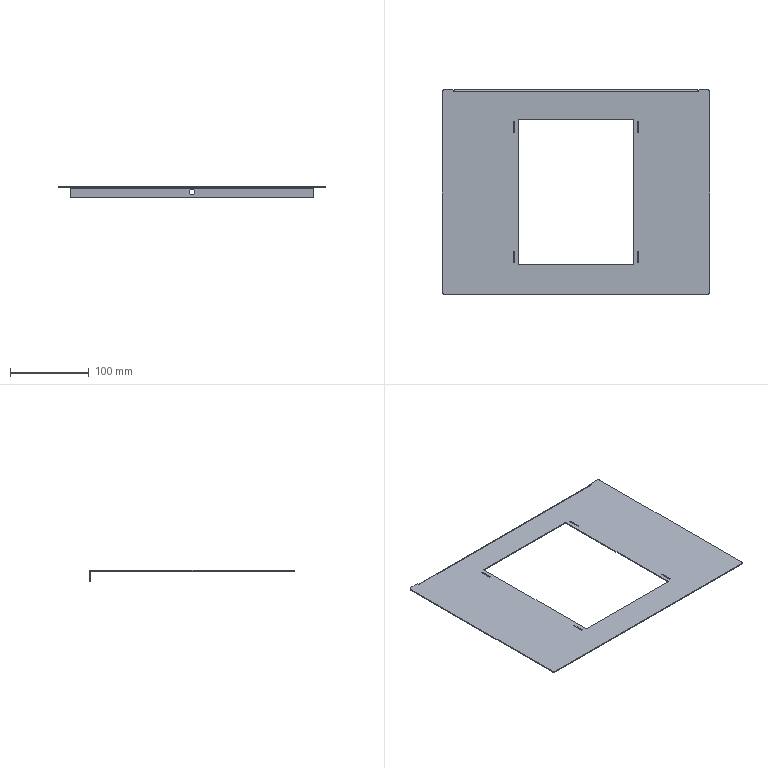Part | SolidWorks | features Cut 2, EdgeFlange 1, FlatPattern 1, ICE 1, SMBaseFlange 1, SheetMetal 1 | 1 solid | 52 faces | box 340 x 260 x 15 mm | volume 78192 mm3 | plane 44 | cylinder 8 | commonest cylinder face diameters 5.4 x5 7 x2 3 x1
STEP:
#1=CARTESIAN_POINT('',(0.,258.8,-2.8));
#2=VERTEX_POINT('',#1);
#3=CARTESIAN_POINT('',(0.,258.8,-9.8));
#4=VERTEX_POINT('',#3);
#5=CARTESIAN_POINT('',(0.,258.8,-6.3));
#6=DIRECTION('',(0.,-1.,0.));
#7=DIRECTION('',(0.,0.,-1.));
#8=AXIS2_PLACEMENT_3D('',#5,#6,#7);
#9=CIRCLE('',#8,3.5);
#10=EDGE_CURVE('',#2,#4,#9,.T.);
#11=ORIENTED_EDGE('',*,*,#10,.T.);
#12=CARTESIAN_POINT('',(0.,260.,-9.8));
#13=VERTEX_POINT('',#12);
#14=CARTESIAN_POINT('',(0.,250.,-9.8));
#15=DIRECTION('',(0.,1.,0.));
#16=VECTOR('',#15,1000.);
#17=LINE('',#14,#16);
#18=EDGE_CURVE('',#4,#13,#17,.T.);
#19=ORIENTED_EDGE('',*,*,#18,.T.);
#20=CARTESIAN_POINT('',(0.,260.,-2.8));
#21=VERTEX_POINT('',#20);
#22=CARTESIAN_POINT('',(0.,260.,-6.3));
#23=DIRECTION('',(0.,1.,0.));
#24=DIRECTION('',(0.,0.,1.));
#25=AXIS2_PLACEMENT_3D('',#22,#23,#24);
#26=CIRCLE('',#25,3.5);
#27=EDGE_CURVE('',#13,#21,#26,.T.);
#28=ORIENTED_EDGE('',*,*,#27,.T.);
#29=CARTESIAN_POINT('',(0.,250.,-2.8));
#30=DIRECTION('',(0.,1.,0.));
#31=VECTOR('',#30,1000.);
#32=LINE('',#29,#31);
#33=EDGE_CURVE('',#2,#21,#32,.T.);
#34=ORIENTED_EDGE('',*,*,#33,.F.);
#35=EDGE_LOOP('',(#11,#19,#28,#34));
#36=FACE_OUTER_BOUND('',#35,.T.);
#37=CARTESIAN_POINT('',(0.,250.,-6.3));
#38=DIRECTION('',(0.,1.,0.));
#39=DIRECTION('',(0.,0.,1.));
#40=AXIS2_PLACEMENT_3D('',#37,#38,#39);
#41=CYLINDRICAL_SURFACE('',#40,3.5);
#42=ADVANCED_FACE('',(#36),#41,.F.);
#43=CARTESIAN_POINT('',(80.,220.,1.2));
#44=VERTEX_POINT('',#43);
#45=CARTESIAN_POINT('',(80.,205.,1.2));
#46=VERTEX_POINT('',#45);
#47=CARTESIAN_POINT('',(80.,205.,1.2));
#48=DIRECTION('',(0.,-1.,0.));
#49=VECTOR('',#48,1000.);
#50=LINE('',#47,#49);
#51=EDGE_CURVE('',#44,#46,#50,.T.);
#52=ORIENTED_EDGE('',*,*,#51,.T.);
#53=CARTESIAN_POINT('',(78.8,205.,1.2));
#54=VERTEX_POINT('',#53);
#55=CARTESIAN_POINT('',(80.,205.,1.2));
#56=DIRECTION('',(-1.,0.,0.));
#57=VECTOR('',#56,1000.);
#58=LINE('',#55,#57);
#59=EDGE_CURVE('',#46,#54,#58,.T.);
#60=ORIENTED_EDGE('',*,*,#59,.T.);
#61=CARTESIAN_POINT('',(78.8,220.,1.2));
#62=VERTEX_POINT('',#61);
#63=CARTESIAN_POINT('',(78.8,205.,1.2));
#64=DIRECTION('',(0.,1.,0.));
#65=VECTOR('',#64,1000.);
#66=LINE('',#63,#65);
#67=EDGE_CURVE('',#54,#62,#66,.T.);
#68=ORIENTED_EDGE('',*,*,#67,.T.);
#69=CARTESIAN_POINT('',(80.,220.,1.2));
#70=DIRECTION('',(1.,0.,0.));
#71=VECTOR('',#70,1000.);
#72=LINE('',#69,#71);
#73=EDGE_CURVE('',#62,#44,#72,.T.);
#74=ORIENTED_EDGE('',*,*,#73,.T.);
#75=EDGE_LOOP('',(#52,#60,#68,#74));
#76=FACE_BOUND('',#75,.T.);
#77=CARTESIAN_POINT('',(78.8,40.,1.2));
#78=VERTEX_POINT('',#77);
#79=CARTESIAN_POINT('',(78.8,55.,1.2));
#80=VERTEX_POINT('',#79);
#81=CARTESIAN_POINT('',(78.8,55.,1.2));
#82=DIRECTION('',(0.,1.,0.));
#83=VECTOR('',#82,1000.);
#84=LINE('',#81,#83);
#85=EDGE_CURVE('',#78,#80,#84,.T.);
#86=ORIENTED_EDGE('',*,*,#85,.T.);
#87=CARTESIAN_POINT('',(80.,55.,1.2));
#88=VERTEX_POINT('',#87);
#89=CARTESIAN_POINT('',(78.8,55.,1.2));
#90=DIRECTION('',(1.,0.,0.));
#91=VECTOR('',#90,1000.);
#92=LINE('',#89,#91);
#93=EDGE_CURVE('',#80,#88,#92,.T.);
#94=ORIENTED_EDGE('',*,*,#93,.T.);
#95=CARTESIAN_POINT('',(80.,40.,1.2));
#96=VERTEX_POINT('',#95);
#97=CARTESIAN_POINT('',(80.,55.,1.2));
#98=DIRECTION('',(0.,-1.,0.));
#99=VECTOR('',#98,1000.);
#100=LINE('',#97,#99);
#101=EDGE_CURVE('',#88,#96,#100,.T.);
#102=ORIENTED_EDGE('',*,*,#101,.T.);
#103=CARTESIAN_POINT('',(78.8,40.,1.2));
#104=DIRECTION('',(-1.,0.,0.));
#105=VECTOR('',#104,1000.);
#106=LINE('',#103,#105);
#107=EDGE_CURVE('',#96,#78,#106,.T.);
#108=ORIENTED_EDGE('',*,*,#107,.T.);
#109=EDGE_LOOP('',(#86,#94,#102,#108));
#110=FACE_BOUND('',#109,.T.);
#111=CARTESIAN_POINT('',(-78.8,55.,1.2));
#112=VERTEX_POINT('',#111);
#113=CARTESIAN_POINT('',(-78.8,40.,1.2));
#114=VERTEX_POINT('',#113);
#115=CARTESIAN_POINT('',(-78.8,40.,1.2));
#116=DIRECTION('',(0.,-1.,0.));
#117=VECTOR('',#116,1000.);
#118=LINE('',#115,#117);
#119=EDGE_CURVE('',#112,#114,#118,.T.);
#120=ORIENTED_EDGE('',*,*,#119,.T.);
#121=CARTESIAN_POINT('',(-80.,40.,1.2));
#122=VERTEX_POINT('',#121);
#123=CARTESIAN_POINT('',(-78.8,40.,1.2));
#124=DIRECTION('',(-1.,0.,0.));
#125=VECTOR('',#124,1000.);
#126=LINE('',#123,#125);
#127=EDGE_CURVE('',#114,#122,#126,.T.);
#128=ORIENTED_EDGE('',*,*,#127,.T.);
#129=CARTESIAN_POINT('',(-80.,55.,1.2));
#130=VERTEX_POINT('',#129);
#131=CARTESIAN_POINT('',(-80.,40.,1.2));
#132=DIRECTION('',(0.,1.,0.));
#133=VECTOR('',#132,1000.);
#134=LINE('',#131,#133);
#135=EDGE_CURVE('',#122,#130,#134,.T.);
#136=ORIENTED_EDGE('',*,*,#135,.T.);
#137=CARTESIAN_POINT('',(-78.8,55.,1.2));
#138=DIRECTION('',(1.,0.,0.));
#139=VECTOR('',#138,1000.);
#140=LINE('',#137,#139);
#141=EDGE_CURVE('',#130,#112,#140,.T.);
#142=ORIENTED_EDGE('',*,*,#141,.T.);
#143=EDGE_LOOP('',(#120,#128,#136,#142));
#144=FACE_BOUND('',#143,.T.);
#145=CARTESIAN_POINT('',(-80.,205.,1.2));
#146=VERTEX_POINT('',#145);
#147=CARTESIAN_POINT('',(-80.,220.,1.2));
#148=VERTEX_POINT('',#147);
#149=CARTESIAN_POINT('',(-80.,220.,1.2));
#150=DIRECTION('',(0.,1.,0.));
#151=VECTOR('',#150,1000.);
#152=LINE('',#149,#151);
#153=EDGE_CURVE('',#146,#148,#152,.T.);
#154=ORIENTED_EDGE('',*,*,#153,.T.);
#155=CARTESIAN_POINT('',(-78.8,220.,1.2));
#156=VERTEX_POINT('',#155);
#157=CARTESIAN_POINT('',(-80.,220.,1.2));
#158=DIRECTION('',(1.,0.,0.));
#159=VECTOR('',#158,1000.);
#160=LINE('',#157,#159);
#161=EDGE_CURVE('',#148,#156,#160,.T.);
#162=ORIENTED_EDGE('',*,*,#161,.T.);
#163=CARTESIAN_POINT('',(-78.8,205.,1.2));
#164=VERTEX_POINT('',#163);
#165=CARTESIAN_POINT('',(-78.8,220.,1.2));
#166=DIRECTION('',(0.,-1.,0.));
#167=VECTOR('',#166,1000.);
#168=LINE('',#165,#167);
#169=EDGE_CURVE('',#156,#164,#168,.T.);
#170=ORIENTED_EDGE('',*,*,#169,.T.);
#171=CARTESIAN_POINT('',(-80.,205.,1.2));
#172=DIRECTION('',(-1.,0.,0.));
#173=VECTOR('',#172,1000.);
#174=LINE('',#171,#173);
#175=EDGE_CURVE('',#164,#146,#174,.T.);
#176=ORIENTED_EDGE('',*,*,#175,.T.);
#177=EDGE_LOOP('',(#154,#162,#170,#176));
#178=FACE_BOUND('',#177,.T.);
#179=CARTESIAN_POINT('',(-73.7,38.,1.2));
#180=VERTEX_POINT('',#179);
#181=CARTESIAN_POINT('',(-73.7,222.,1.2));
#182=VERTEX_POINT('',#181);
#183=CARTESIAN_POINT('',(-73.7,38.,1.2));
#184=DIRECTION('',(0.,1.,0.));
#185=VECTOR('',#184,1000.);
#186=LINE('',#183,#185);
#187=EDGE_CURVE('',#180,#182,#186,.T.);
#188=ORIENTED_EDGE('',*,*,#187,.T.);
#189=CARTESIAN_POINT('',(73.7,222.,1.2));
#190=VERTEX_POINT('',#189);
#191=CARTESIAN_POINT('',(-73.7,222.,1.2));
#192=DIRECTION('',(1.,0.,0.));
#193=VECTOR('',#192,1000.);
#194=LINE('',#191,#193);
#195=EDGE_CURVE('',#182,#190,#194,.T.);
#196=ORIENTED_EDGE('',*,*,#195,.T.);
#197=CARTESIAN_POINT('',(73.7,38.,1.2));
#198=VERTEX_POINT('',#197);
#199=CARTESIAN_POINT('',(73.7,38.,1.2));
#200=DIRECTION('',(0.,-1.,0.));
#201=VECTOR('',#200,1000.);
#202=LINE('',#199,#201);
#203=EDGE_CURVE('',#190,#198,#202,.T.);
#204=ORIENTED_EDGE('',*,*,#203,.T.);
#205=CARTESIAN_POINT('',(-73.7,38.,1.2));
#206=DIRECTION('',(-1.,0.,0.));
#207=VECTOR('',#206,1000.);
#208=LINE('',#205,#207);
#209=EDGE_CURVE('',#198,#180,#208,.T.);
#210=ORIENTED_EDGE('',*,*,#209,.T.);
#211=EDGE_LOOP('',(#188,#196,#204,#210));
#212=FACE_BOUND('',#211,.T.);
#213=CARTESIAN_POINT('',(155.,260.,1.2));
#214=VERTEX_POINT('',#213);
#215=CARTESIAN_POINT('',(155.,258.8,1.2));
#216=VERTEX_POINT('',#215);
#217=CARTESIAN_POINT('',(155.,258.8,1.2));
#218=DIRECTION('',(0.,-1.,0.));
#219=VECTOR('',#218,1000.);
#220=LINE('',#217,#219);
#221=EDGE_CURVE('',#214,#216,#220,.T.);
#222=ORIENTED_EDGE('',*,*,#221,.T.);
#223=CARTESIAN_POINT('',(155.12,258.8,1.2));
#224=VERTEX_POINT('',#223);
#225=CARTESIAN_POINT('',(167.3,258.8,1.2));
#226=DIRECTION('',(1.,0.,0.));
#227=VECTOR('',#226,1000.);
#228=LINE('',#225,#227);
#229=EDGE_CURVE('',#216,#224,#228,.T.);
#230=ORIENTED_EDGE('',*,*,#229,.T.);
#231=CARTESIAN_POINT('',(155.12,257.18,1.2));
#232=VERTEX_POINT('',#231);
#233=CARTESIAN_POINT('',(155.12,257.3,1.2));
#234=DIRECTION('',(0.,-1.,0.));
#235=VECTOR('',#234,1000.);
#236=LINE('',#233,#235);
#237=EDGE_CURVE('',#224,#232,#236,.T.);
#238=ORIENTED_EDGE('',*,*,#237,.T.);
#239=CARTESIAN_POINT('',(155.,257.18,1.2));
#240=VERTEX_POINT('',#239);
#241=CARTESIAN_POINT('',(167.3,257.18,1.2));
#242=DIRECTION('',(-1.,0.,0.));
#243=VECTOR('',#242,1000.);
#244=LINE('',#241,#243);
#245=EDGE_CURVE('',#232,#240,#244,.T.);
#246=ORIENTED_EDGE('',*,*,#245,.T.);
#247=CARTESIAN_POINT('',(155.,257.3,1.2));
#248=VERTEX_POINT('',#247);
#249=CARTESIAN_POINT('',(155.,257.3,1.2));
#250=DIRECTION('',(0.,1.,0.));
#251=VECTOR('',#250,1000.);
#252=LINE('',#249,#251);
#253=EDGE_CURVE('',#240,#248,#252,.T.);
#254=ORIENTED_EDGE('',*,*,#253,.T.);
#255=CARTESIAN_POINT('',(-155.,257.3,1.2));
#256=VERTEX_POINT('',#255);
#257=CARTESIAN_POINT('',(155.,257.3,1.2));
#258=DIRECTION('',(-1.,0.,0.));
#259=VECTOR('',#258,1000.);
#260=LINE('',#257,#259);
#261=EDGE_CURVE('',#248,#256,#260,.T.);
#262=ORIENTED_EDGE('',*,*,#261,.T.);
#263=CARTESIAN_POINT('',(-155.,257.18,1.2));
#264=VERTEX_POINT('',#263);
#265=CARTESIAN_POINT('',(-155.,257.3,1.2));
#266=DIRECTION('',(0.,-1.,0.));
#267=VECTOR('',#266,1000.);
#268=LINE('',#265,#267);
#269=EDGE_CURVE('',#256,#264,#268,.T.);
#270=ORIENTED_EDGE('',*,*,#269,.T.);
#271=CARTESIAN_POINT('',(-155.12,257.18,1.2));
#272=VERTEX_POINT('',#271);
#273=CARTESIAN_POINT('',(167.3,257.18,1.2));
#274=DIRECTION('',(-1.,0.,0.));
#275=VECTOR('',#274,1000.);
#276=LINE('',#273,#275);
#277=EDGE_CURVE('',#264,#272,#276,.T.);
#278=ORIENTED_EDGE('',*,*,#277,.T.);
#279=CARTESIAN_POINT('',(-155.12,258.8,1.2));
#280=VERTEX_POINT('',#279);
#281=CARTESIAN_POINT('',(-155.12,257.3,1.2));
#282=DIRECTION('',(0.,1.,0.));
#283=VECTOR('',#282,1000.);
#284=LINE('',#281,#283);
#285=EDGE_CURVE('',#272,#280,#284,.T.);
#286=ORIENTED_EDGE('',*,*,#285,.T.);
#287=CARTESIAN_POINT('',(-155.,258.8,1.2));
#288=VERTEX_POINT('',#287);
#289=CARTESIAN_POINT('',(167.3,258.8,1.2));
#290=DIRECTION('',(1.,0.,0.));
#291=VECTOR('',#290,1000.);
#292=LINE('',#289,#291);
#293=EDGE_CURVE('',#280,#288,#292,.T.);
#294=ORIENTED_EDGE('',*,*,#293,.T.);
#295=CARTESIAN_POINT('',(-155.,260.,1.2));
#296=VERTEX_POINT('',#295);
#297=CARTESIAN_POINT('',(-155.,260.,1.2));
#298=DIRECTION('',(0.,1.,0.));
#299=VECTOR('',#298,1000.);
#300=LINE('',#297,#299);
#301=EDGE_CURVE('',#288,#296,#300,.T.);
#302=ORIENTED_EDGE('',*,*,#301,.T.);
#303=CARTESIAN_POINT('',(-167.3,260.,1.2));
#304=VERTEX_POINT('',#303);
#305=CARTESIAN_POINT('',(-167.3,260.,1.2));
#306=DIRECTION('',(-1.,0.,0.));
#307=VECTOR('',#306,1000.);
#308=LINE('',#305,#307);
#309=EDGE_CURVE('',#296,#304,#308,.T.);
#310=ORIENTED_EDGE('',*,*,#309,.T.);
#311=CARTESIAN_POINT('',(-170.,257.3,1.2));
#312=VERTEX_POINT('',#311);
#313=CARTESIAN_POINT('',(-167.3,257.3,1.2));
#314=DIRECTION('',(0.,0.,1.));
#315=DIRECTION('',(1.,0.,0.));
#316=AXIS2_PLACEMENT_3D('',#313,#314,#315);
#317=CIRCLE('',#316,2.7);
#318=EDGE_CURVE('',#304,#312,#317,.T.);
#319=ORIENTED_EDGE('',*,*,#318,.T.);
#320=CARTESIAN_POINT('',(-170.,2.7,1.2));
#321=VERTEX_POINT('',#320);
#322=CARTESIAN_POINT('',(-170.,257.3,1.2));
#323=DIRECTION('',(0.,-1.,0.));
#324=VECTOR('',#323,1000.);
#325=LINE('',#322,#324);
#326=EDGE_CURVE('',#312,#321,#325,.T.);
#327=ORIENTED_EDGE('',*,*,#326,.T.);
#328=CARTESIAN_POINT('',(-167.3,0.,1.2));
#329=VERTEX_POINT('',#328);
#330=CARTESIAN_POINT('',(-167.3,2.7,1.2));
#331=DIRECTION('',(0.,0.,1.));
#332=DIRECTION('',(1.,0.,0.));
#333=AXIS2_PLACEMENT_3D('',#330,#331,#332);
#334=CIRCLE('',#333,2.7);
#335=EDGE_CURVE('',#321,#329,#334,.T.);
#336=ORIENTED_EDGE('',*,*,#335,.T.);
#337=CARTESIAN_POINT('',(167.3,0.,1.2));
#338=VERTEX_POINT('',#337);
#339=CARTESIAN_POINT('',(-167.3,0.,1.2));
#340=DIRECTION('',(1.,0.,0.));
#341=VECTOR('',#340,1000.);
#342=LINE('',#339,#341);
#343=EDGE_CURVE('',#329,#338,#342,.T.);
#344=ORIENTED_EDGE('',*,*,#343,.T.);
#345=CARTESIAN_POINT('',(170.,2.7,1.2));
#346=VERTEX_POINT('',#345);
#347=CARTESIAN_POINT('',(167.3,2.7,1.2));
#348=DIRECTION('',(0.,0.,1.));
#349=DIRECTION('',(1.,0.,0.));
#350=AXIS2_PLACEMENT_3D('',#347,#348,#349);
#351=CIRCLE('',#350,2.7);
#352=EDGE_CURVE('',#338,#346,#351,.T.);
#353=ORIENTED_EDGE('',*,*,#352,.T.);
#354=CARTESIAN_POINT('',(170.,257.3,1.2));
#355=VERTEX_POINT('',#354);
#356=CARTESIAN_POINT('',(170.,2.7,1.2));
#357=DIRECTION('',(0.,1.,0.));
#358=VECTOR('',#357,1000.);
#359=LINE('',#356,#358);
#360=EDGE_CURVE('',#346,#355,#359,.T.);
#361=ORIENTED_EDGE('',*,*,#360,.T.);
#362=CARTESIAN_POINT('',(167.3,260.,1.2));
#363=VERTEX_POINT('',#362);
#364=CARTESIAN_POINT('',(167.3,257.3,1.2));
#365=DIRECTION('',(0.,0.,1.));
#366=DIRECTION('',(1.,0.,0.));
#367=AXIS2_PLACEMENT_3D('',#364,#365,#366);
#368=CIRCLE('',#367,2.7);
#369=EDGE_CURVE('',#355,#363,#368,.T.);
#370=ORIENTED_EDGE('',*,*,#369,.T.);
#371=CARTESIAN_POINT('',(155.,260.,1.2));
#372=DIRECTION('',(-1.,0.,0.));
#373=VECTOR('',#372,1000.);
#374=LINE('',#371,#373);
#375=EDGE_CURVE('',#363,#214,#374,.T.);
#376=ORIENTED_EDGE('',*,*,#375,.T.);
#377=EDGE_LOOP('',(#222,#230,#238,#246,#254,#262,#270,#278,#286,#294,#302,#310,#319,#327,#336,#344,#353,#361,#370,#376));
#378=FACE_OUTER_BOUND('',#377,.T.);
#379=CARTESIAN_POINT('',(167.3,257.3,1.2));
#380=DIRECTION('',(0.,0.,1.));
#381=DIRECTION('',(1.,0.,0.));
#382=AXIS2_PLACEMENT_3D('',#379,#380,#381);
#383=PLANE('',#382);
#384=ADVANCED_FACE('',(#76,#110,#144,#178,#212,#378),#383,.T.);
#385=CARTESIAN_POINT('',(80.,205.,0.));
#386=VERTEX_POINT('',#385);
#387=CARTESIAN_POINT('',(78.8,205.,0.));
#388=VERTEX_POINT('',#387);
#389=CARTESIAN_POINT('',(80.,205.,0.));
#390=DIRECTION('',(-1.,0.,0.));
#391=VECTOR('',#390,1000.);
#392=LINE('',#389,#391);
#393=EDGE_CURVE('',#386,#388,#392,.T.);
#394=ORIENTED_EDGE('',*,*,#393,.F.);
#395=CARTESIAN_POINT('',(80.,220.,0.));
#396=VERTEX_POINT('',#395);
#397=CARTESIAN_POINT('',(80.,205.,0.));
#398=DIRECTION('',(0.,-1.,0.));
#399=VECTOR('',#398,1000.);
#400=LINE('',#397,#399);
#401=EDGE_CURVE('',#396,#386,#400,.T.);
#402=ORIENTED_EDGE('',*,*,#401,.F.);
#403=CARTESIAN_POINT('',(78.8,220.,0.));
#404=VERTEX_POINT('',#403);
#405=CARTESIAN_POINT('',(80.,220.,0.));
#406=DIRECTION('',(1.,0.,0.));
#407=VECTOR('',#406,1000.);
#408=LINE('',#405,#407);
#409=EDGE_CURVE('',#404,#396,#408,.T.);
#410=ORIENTED_EDGE('',*,*,#409,.F.);
#411=CARTESIAN_POINT('',(78.8,205.,0.));
#412=DIRECTION('',(0.,1.,0.));
#413=VECTOR('',#412,1000.);
#414=LINE('',#411,#413);
#415=EDGE_CURVE('',#388,#404,#414,.T.);
#416=ORIENTED_EDGE('',*,*,#415,.F.);
#417=EDGE_LOOP('',(#394,#402,#410,#416));
#418=FACE_BOUND('',#417,.T.);
#419=CARTESIAN_POINT('',(78.8,55.,0.));
#420=VERTEX_POINT('',#419);
#421=CARTESIAN_POINT('',(80.,55.,0.));
#422=VERTEX_POINT('',#421);
#423=CARTESIAN_POINT('',(78.8,55.,0.));
#424=DIRECTION('',(1.,0.,0.));
#425=VECTOR('',#424,1000.);
#426=LINE('',#423,#425);
#427=EDGE_CURVE('',#420,#422,#426,.T.);
#428=ORIENTED_EDGE('',*,*,#427,.F.);
#429=CARTESIAN_POINT('',(78.8,40.,0.));
#430=VERTEX_POINT('',#429);
#431=CARTESIAN_POINT('',(78.8,55.,0.));
#432=DIRECTION('',(0.,1.,0.));
#433=VECTOR('',#432,1000.);
#434=LINE('',#431,#433);
#435=EDGE_CURVE('',#430,#420,#434,.T.);
#436=ORIENTED_EDGE('',*,*,#435,.F.);
#437=CARTESIAN_POINT('',(80.,40.,0.));
#438=VERTEX_POINT('',#437);
#439=CARTESIAN_POINT('',(78.8,40.,0.));
#440=DIRECTION('',(-1.,0.,0.));
#441=VECTOR('',#440,1000.);
#442=LINE('',#439,#441);
#443=EDGE_CURVE('',#438,#430,#442,.T.);
#444=ORIENTED_EDGE('',*,*,#443,.F.);
#445=CARTESIAN_POINT('',(80.,55.,0.));
#446=DIRECTION('',(0.,-1.,0.));
#447=VECTOR('',#446,1000.);
#448=LINE('',#445,#447);
#449=EDGE_CURVE('',#422,#438,#448,.T.);
#450=ORIENTED_EDGE('',*,*,#449,.F.);
#451=EDGE_LOOP('',(#428,#436,#444,#450));
#452=FACE_BOUND('',#451,.T.);
#453=CARTESIAN_POINT('',(-78.8,40.,0.));
#454=VERTEX_POINT('',#453);
#455=CARTESIAN_POINT('',(-80.,40.,0.));
#456=VERTEX_POINT('',#455);
#457=CARTESIAN_POINT('',(-78.8,40.,0.));
#458=DIRECTION('',(-1.,0.,0.));
#459=VECTOR('',#458,1000.);
#460=LINE('',#457,#459);
#461=EDGE_CURVE('',#454,#456,#460,.T.);
#462=ORIENTED_EDGE('',*,*,#461,.F.);
#463=CARTESIAN_POINT('',(-78.8,55.,0.));
#464=VERTEX_POINT('',#463);
#465=CARTESIAN_POINT('',(-78.8,40.,0.));
#466=DIRECTION('',(0.,-1.,0.));
#467=VECTOR('',#466,1000.);
#468=LINE('',#465,#467);
#469=EDGE_CURVE('',#464,#454,#468,.T.);
#470=ORIENTED_EDGE('',*,*,#469,.F.);
#471=CARTESIAN_POINT('',(-80.,55.,0.));
#472=VERTEX_POINT('',#471);
#473=CARTESIAN_POINT('',(-78.8,55.,0.));
#474=DIRECTION('',(1.,0.,0.));
#475=VECTOR('',#474,1000.);
#476=LINE('',#473,#475);
#477=EDGE_CURVE('',#472,#464,#476,.T.);
#478=ORIENTED_EDGE('',*,*,#477,.F.);
#479=CARTESIAN_POINT('',(-80.,40.,0.));
#480=DIRECTION('',(0.,1.,0.));
#481=VECTOR('',#480,1000.);
#482=LINE('',#479,#481);
#483=EDGE_CURVE('',#456,#472,#482,.T.);
#484=ORIENTED_EDGE('',*,*,#483,.F.);
#485=EDGE_LOOP('',(#462,#470,#478,#484));
#486=FACE_BOUND('',#485,.T.);
#487=CARTESIAN_POINT('',(-80.,220.,0.));
#488=VERTEX_POINT('',#487);
#489=CARTESIAN_POINT('',(-78.8,220.,0.));
#490=VERTEX_POINT('',#489);
#491=CARTESIAN_POINT('',(-80.,220.,0.));
#492=DIRECTION('',(1.,0.,0.));
#493=VECTOR('',#492,1000.);
#494=LINE('',#491,#493);
#495=EDGE_CURVE('',#488,#490,#494,.T.);
#496=ORIENTED_EDGE('',*,*,#495,.F.);
#497=CARTESIAN_POINT('',(-80.,205.,0.));
#498=VERTEX_POINT('',#497);
#499=CARTESIAN_POINT('',(-80.,220.,0.));
#500=DIRECTION('',(0.,1.,0.));
#501=VECTOR('',#500,1000.);
#502=LINE('',#499,#501);
#503=EDGE_CURVE('',#498,#488,#502,.T.);
#504=ORIENTED_EDGE('',*,*,#503,.F.);
#505=CARTESIAN_POINT('',(-78.8,205.,0.));
#506=VERTEX_POINT('',#505);
#507=CARTESIAN_POINT('',(-80.,205.,0.));
#508=DIRECTION('',(-1.,0.,0.));
#509=VECTOR('',#508,1000.);
#510=LINE('',#507,#509);
#511=EDGE_CURVE('',#506,#498,#510,.T.);
#512=ORIENTED_EDGE('',*,*,#511,.F.);
#513=CARTESIAN_POINT('',(-78.8,220.,0.));
#514=DIRECTION('',(0.,-1.,0.));
#515=VECTOR('',#514,1000.);
#516=LINE('',#513,#515);
#517=EDGE_CURVE('',#490,#506,#516,.T.);
#518=ORIENTED_EDGE('',*,*,#517,.F.);
#519=EDGE_LOOP('',(#496,#504,#512,#518));
#520=FACE_BOUND('',#519,.T.);
#521=CARTESIAN_POINT('',(-73.7,222.,0.));
#522=VERTEX_POINT('',#521);
#523=CARTESIAN_POINT('',(73.7,222.,0.));
#524=VERTEX_POINT('',#523);
#525=CARTESIAN_POINT('',(-73.7,222.,0.));
#526=DIRECTION('',(1.,0.,0.));
#527=VECTOR('',#526,1000.);
#528=LINE('',#525,#527);
#529=EDGE_CURVE('',#522,#524,#528,.T.);
#530=ORIENTED_EDGE('',*,*,#529,.F.);
#531=CARTESIAN_POINT('',(-73.7,38.,0.));
#532=VERTEX_POINT('',#531);
#533=CARTESIAN_POINT('',(-73.7,38.,0.));
#534=DIRECTION('',(0.,1.,0.));
#535=VECTOR('',#534,1000.);
#536=LINE('',#533,#535);
#537=EDGE_CURVE('',#532,#522,#536,.T.);
#538=ORIENTED_EDGE('',*,*,#537,.F.);
#539=CARTESIAN_POINT('',(73.7,38.,0.));
#540=VERTEX_POINT('',#539);
#541=CARTESIAN_POINT('',(-73.7,38.,0.));
#542=DIRECTION('',(-1.,0.,0.));
#543=VECTOR('',#542,1000.);
#544=LINE('',#541,#543);
#545=EDGE_CURVE('',#540,#532,#544,.T.);
#546=ORIENTED_EDGE('',*,*,#545,.F.);
#547=CARTESIAN_POINT('',(73.7,38.,0.));
#548=DIRECTION('',(0.,-1.,0.));
#549=VECTOR('',#548,1000.);
#550=LINE('',#547,#549);
#551=EDGE_CURVE('',#524,#540,#550,.T.);
#552=ORIENTED_EDGE('',*,*,#551,.F.);
#553=EDGE_LOOP('',(#530,#538,#546,#552));
#554=FACE_BOUND('',#553,.T.);
#555=CARTESIAN_POINT('',(155.,258.8,0.));
#556=VERTEX_POINT('',#555);
#557=CARTESIAN_POINT('',(155.12,258.8,0.));
#558=VERTEX_POINT('',#557);
#559=CARTESIAN_POINT('',(155.,258.8,0.));
#560=DIRECTION('',(1.,0.,0.));
#561=VECTOR('',#560,1000.);
#562=LINE('',#559,#561);
#563=EDGE_CURVE('',#556,#558,#562,.T.);
#564=ORIENTED_EDGE('',*,*,#563,.F.);
#565=CARTESIAN_POINT('',(155.,260.,0.));
#566=VERTEX_POINT('',#565);
#567=CARTESIAN_POINT('',(155.,258.8,0.));
#568=DIRECTION('',(0.,-1.,0.));
#569=VECTOR('',#568,1000.);
#570=LINE('',#567,#569);
#571=EDGE_CURVE('',#566,#556,#570,.T.);
#572=ORIENTED_EDGE('',*,*,#571,.F.);
#573=CARTESIAN_POINT('',(167.3,260.,0.));
#574=VERTEX_POINT('',#573);
#575=CARTESIAN_POINT('',(155.,260.,0.));
#576=DIRECTION('',(-1.,0.,0.));
#577=VECTOR('',#576,1000.);
#578=LINE('',#575,#577);
#579=EDGE_CURVE('',#574,#566,#578,.T.);
#580=ORIENTED_EDGE('',*,*,#579,.F.);
#581=CARTESIAN_POINT('',(170.,257.3,0.));
#582=VERTEX_POINT('',#581);
#583=CARTESIAN_POINT('',(167.3,257.3,0.));
#584=DIRECTION('',(0.,0.,1.));
#585=DIRECTION('',(1.,0.,0.));
#586=AXIS2_PLACEMENT_3D('',#583,#584,#585);
#587=CIRCLE('',#586,2.7);
#588=EDGE_CURVE('',#582,#574,#587,.T.);
#589=ORIENTED_EDGE('',*,*,#588,.F.);
#590=CARTESIAN_POINT('',(170.,2.7,0.));
#591=VERTEX_POINT('',#590);
#592=CARTESIAN_POINT('',(170.,2.7,0.));
#593=DIRECTION('',(0.,1.,0.));
#594=VECTOR('',#593,1000.);
#595=LINE('',#592,#594);
#596=EDGE_CURVE('',#591,#582,#595,.T.);
#597=ORIENTED_EDGE('',*,*,#596,.F.);
#598=CARTESIAN_POINT('',(167.3,0.,0.));
#599=VERTEX_POINT('',#598);
#600=CARTESIAN_POINT('',(167.3,2.7,0.));
#601=DIRECTION('',(0.,0.,1.));
#602=DIRECTION('',(1.,0.,0.));
#603=AXIS2_PLACEMENT_3D('',#600,#601,#602);
#604=CIRCLE('',#603,2.7);
#605=EDGE_CURVE('',#599,#591,#604,.T.);
#606=ORIENTED_EDGE('',*,*,#605,.F.);
#607=CARTESIAN_POINT('',(-167.3,0.,0.));
#608=VERTEX_POINT('',#607);
#609=CARTESIAN_POINT('',(-167.3,0.,0.));
#610=DIRECTION('',(1.,0.,0.));
#611=VECTOR('',#610,1000.);
#612=LINE('',#609,#611);
#613=EDGE_CURVE('',#608,#599,#612,.T.);
#614=ORIENTED_EDGE('',*,*,#613,.F.);
#615=CARTESIAN_POINT('',(-170.,2.7,0.));
#616=VERTEX_POINT('',#615);
#617=CARTESIAN_POINT('',(-167.3,2.7,0.));
#618=DIRECTION('',(0.,0.,1.));
#619=DIRECTION('',(1.,0.,0.));
#620=AXIS2_PLACEMENT_3D('',#617,#618,#619);
#621=CIRCLE('',#620,2.7);
#622=EDGE_CURVE('',#616,#608,#621,.T.);
#623=ORIENTED_EDGE('',*,*,#622,.F.);
#624=CARTESIAN_POINT('',(-170.,257.3,0.));
#625=VERTEX_POINT('',#624);
#626=CARTESIAN_POINT('',(-170.,257.3,0.));
#627=DIRECTION('',(0.,-1.,0.));
#628=VECTOR('',#627,1000.);
#629=LINE('',#626,#628);
#630=EDGE_CURVE('',#625,#616,#629,.T.);
#631=ORIENTED_EDGE('',*,*,#630,.F.);
#632=CARTESIAN_POINT('',(-167.3,260.,0.));
#633=VERTEX_POINT('',#632);
#634=CARTESIAN_POINT('',(-167.3,257.3,0.));
#635=DIRECTION('',(0.,0.,1.));
#636=DIRECTION('',(1.,0.,0.));
#637=AXIS2_PLACEMENT_3D('',#634,#635,#636);
#638=CIRCLE('',#637,2.7);
#639=EDGE_CURVE('',#633,#625,#638,.T.);
#640=ORIENTED_EDGE('',*,*,#639,.F.);
#641=CARTESIAN_POINT('',(-155.,260.,0.));
#642=VERTEX_POINT('',#641);
#643=CARTESIAN_POINT('',(-167.3,260.,0.));
#644=DIRECTION('',(-1.,0.,0.));
#645=VECTOR('',#644,1000.);
#646=LINE('',#643,#645);
#647=EDGE_CURVE('',#642,#633,#646,.T.);
#648=ORIENTED_EDGE('',*,*,#647,.F.);
#649=CARTESIAN_POINT('',(-155.,258.8,0.));
#650=VERTEX_POINT('',#649);
#651=CARTESIAN_POINT('',(-155.,260.,0.));
#652=DIRECTION('',(0.,1.,0.));
#653=VECTOR('',#652,1000.);
#654=LINE('',#651,#653);
#655=EDGE_CURVE('',#650,#642,#654,.T.);
#656=ORIENTED_EDGE('',*,*,#655,.F.);
#657=CARTESIAN_POINT('',(-155.12,258.8,0.));
#658=VERTEX_POINT('',#657);
#659=CARTESIAN_POINT('',(-155.12,258.8,0.));
#660=DIRECTION('',(1.,0.,0.));
#661=VECTOR('',#660,1000.);
#662=LINE('',#659,#661);
#663=EDGE_CURVE('',#658,#650,#662,.T.);
#664=ORIENTED_EDGE('',*,*,#663,.F.);
#665=CARTESIAN_POINT('',(-155.12,257.18,0.));
#666=VERTEX_POINT('',#665);
#667=CARTESIAN_POINT('',(-155.12,257.18,0.));
#668=DIRECTION('',(0.,1.,0.));
#669=VECTOR('',#668,1000.);
#670=LINE('',#667,#669);
#671=EDGE_CURVE('',#666,#658,#670,.T.);
#672=ORIENTED_EDGE('',*,*,#671,.F.);
#673=CARTESIAN_POINT('',(-155.,257.18,0.));
#674=VERTEX_POINT('',#673);
#675=CARTESIAN_POINT('',(-155.,257.18,0.));
#676=DIRECTION('',(-1.,0.,0.));
#677=VECTOR('',#676,1000.);
#678=LINE('',#675,#677);
#679=EDGE_CURVE('',#674,#666,#678,.T.);
#680=ORIENTED_EDGE('',*,*,#679,.F.);
#681=CARTESIAN_POINT('',(-155.,257.3,0.));
#682=VERTEX_POINT('',#681);
#683=CARTESIAN_POINT('',(-155.,257.3,0.));
#684=DIRECTION('',(0.,-1.,0.));
#685=VECTOR('',#684,1000.);
#686=LINE('',#683,#685);
#687=EDGE_CURVE('',#682,#674,#686,.T.);
#688=ORIENTED_EDGE('',*,*,#687,.F.);
#689=CARTESIAN_POINT('',(155.,257.3,0.));
#690=VERTEX_POINT('',#689);
#691=CARTESIAN_POINT('',(155.,257.3,0.));
#692=DIRECTION('',(-1.,0.,0.));
#693=VECTOR('',#692,1000.);
#694=LINE('',#691,#693);
#695=EDGE_CURVE('',#690,#682,#694,.T.);
#696=ORIENTED_EDGE('',*,*,#695,.F.);
#697=CARTESIAN_POINT('',(155.,257.18,0.));
#698=VERTEX_POINT('',#697);
#699=CARTESIAN_POINT('',(155.,257.18,0.));
#700=DIRECTION('',(0.,1.,0.));
#701=VECTOR('',#700,1000.);
#702=LINE('',#699,#701);
#703=EDGE_CURVE('',#698,#690,#702,.T.);
#704=ORIENTED_EDGE('',*,*,#703,.F.);
#705=CARTESIAN_POINT('',(155.12,257.18,0.));
#706=VERTEX_POINT('',#705);
#707=CARTESIAN_POINT('',(155.12,257.18,0.));
#708=DIRECTION('',(-1.,0.,0.));
#709=VECTOR('',#708,1000.);
#710=LINE('',#707,#709);
#711=EDGE_CURVE('',#706,#698,#710,.T.);
#712=ORIENTED_EDGE('',*,*,#711,.F.);
#713=CARTESIAN_POINT('',(155.12,258.8,0.));
#714=DIRECTION('',(0.,-1.,0.));
#715=VECTOR('',#714,1000.);
#716=LINE('',#713,#715);
#717=EDGE_CURVE('',#558,#706,#716,.T.);
#718=ORIENTED_EDGE('',*,*,#717,.F.);
#719=EDGE_LOOP('',(#564,#572,#580,#589,#597,#606,#614,#623,#631,#640,#648,#656,#664,#672,#680,#688,#696,#704,#712,#718));
#720=FACE_OUTER_BOUND('',#719,.T.);
#721=CARTESIAN_POINT('',(167.3,257.3,0.));
#722=DIRECTION('',(0.,0.,1.));
#723=DIRECTION('',(1.,0.,0.));
#724=AXIS2_PLACEMENT_3D('',#721,#722,#723);
#725=PLANE('',#724);
#726=ADVANCED_FACE('',(#418,#452,#486,#520,#554,#720),#725,.F.);
#727=ORIENTED_EDGE('',*,*,#571,.T.);
#728=CARTESIAN_POINT('',(155.,258.8,1.2));
#729=DIRECTION('',(0.,0.,-1.));
#730=VECTOR('',#729,1000.);
#731=LINE('',#728,#730);
#732=EDGE_CURVE('',#216,#556,#731,.T.);
#733=ORIENTED_EDGE('',*,*,#732,.F.);
#734=ORIENTED_EDGE('',*,*,#221,.F.);
#735=CARTESIAN_POINT('',(155.,260.,1.2));
#736=DIRECTION('',(0.,0.,-1.));
#737=VECTOR('',#736,1000.);
#738=LINE('',#735,#737);
#739=EDGE_CURVE('',#214,#566,#738,.T.);
#740=ORIENTED_EDGE('',*,*,#739,.T.);
#741=EDGE_LOOP('',(#727,#733,#734,#740));
#742=FACE_OUTER_BOUND('',#741,.T.);
#743=CARTESIAN_POINT('',(155.,258.8,1.2));
#744=DIRECTION('',(1.,0.,0.));
#745=DIRECTION('',(0.,0.,-1.));
#746=AXIS2_PLACEMENT_3D('',#743,#744,#745);
#747=PLANE('',#746);
#748=ADVANCED_FACE('',(#742),#747,.F.);
#749=ORIENTED_EDGE('',*,*,#655,.T.);
#750=CARTESIAN_POINT('',(-155.,260.,1.2));
#751=DIRECTION('',(0.,0.,-1.));
#752=VECTOR('',#751,1000.);
#753=LINE('',#750,#752);
#754=EDGE_CURVE('',#296,#642,#753,.T.);
#755=ORIENTED_EDGE('',*,*,#754,.F.);
#756=ORIENTED_EDGE('',*,*,#301,.F.);
#757=CARTESIAN_POINT('',(-155.,258.8,1.2));
#758=DIRECTION('',(0.,0.,-1.));
#759=VECTOR('',#758,1000.);
#760=LINE('',#757,#759);
#761=EDGE_CURVE('',#288,#650,#760,.T.);
#762=ORIENTED_EDGE('',*,*,#761,.T.);
#763=EDGE_LOOP('',(#749,#755,#756,#762));
#764=FACE_OUTER_BOUND('',#763,.T.);
#765=CARTESIAN_POINT('',(-155.,260.,1.2));
#766=DIRECTION('',(-1.,0.,0.));
#767=DIRECTION('',(0.,0.,1.));
#768=AXIS2_PLACEMENT_3D('',#765,#766,#767);
#769=PLANE('',#768);
#770=ADVANCED_FACE('',(#764),#769,.F.);
#771=ORIENTED_EDGE('',*,*,#647,.T.);
#772=CARTESIAN_POINT('',(-167.3,260.,1.2));
#773=DIRECTION('',(0.,0.,-1.));
#774=VECTOR('',#773,1000.);
#775=LINE('',#772,#774);
#776=EDGE_CURVE('',#304,#633,#775,.T.);
#777=ORIENTED_EDGE('',*,*,#776,.F.);
#778=ORIENTED_EDGE('',*,*,#309,.F.);
#779=ORIENTED_EDGE('',*,*,#754,.T.);
#780=EDGE_LOOP('',(#771,#777,#778,#779));
#781=FACE_OUTER_BOUND('',#780,.T.);
#782=CARTESIAN_POINT('',(-167.3,260.,1.2));
#783=DIRECTION('',(0.,-1.,0.));
#784=DIRECTION('',(1.,0.,0.));
#785=AXIS2_PLACEMENT_3D('',#782,#783,#784);
#786=PLANE('',#785);
#787=ADVANCED_FACE('',(#781),#786,.F.);
#788=ORIENTED_EDGE('',*,*,#639,.T.);
#789=CARTESIAN_POINT('',(-170.,257.3,1.2));
#790=DIRECTION('',(0.,0.,-1.));
#791=VECTOR('',#790,1000.);
#792=LINE('',#789,#791);
#793=EDGE_CURVE('',#312,#625,#792,.T.);
#794=ORIENTED_EDGE('',*,*,#793,.F.);
#795=ORIENTED_EDGE('',*,*,#318,.F.);
#796=ORIENTED_EDGE('',*,*,#776,.T.);
#797=EDGE_LOOP('',(#788,#794,#795,#796));
#798=FACE_OUTER_BOUND('',#797,.T.);
#799=CARTESIAN_POINT('',(-167.3,257.3,1.2));
#800=DIRECTION('',(0.,0.,-1.));
#801=DIRECTION('',(-1.,0.,0.));
#802=AXIS2_PLACEMENT_3D('',#799,#800,#801);
#803=CYLINDRICAL_SURFACE('',#802,2.7);
#804=ADVANCED_FACE('',(#798),#803,.T.);
#805=ORIENTED_EDGE('',*,*,#630,.T.);
#806=CARTESIAN_POINT('',(-170.,2.7,1.2));
#807=DIRECTION('',(0.,0.,-1.));
#808=VECTOR('',#807,1000.);
#809=LINE('',#806,#808);
#810=EDGE_CURVE('',#321,#616,#809,.T.);
#811=ORIENTED_EDGE('',*,*,#810,.F.);
#812=ORIENTED_EDGE('',*,*,#326,.F.);
#813=ORIENTED_EDGE('',*,*,#793,.T.);
#814=EDGE_LOOP('',(#805,#811,#812,#813));
#815=FACE_OUTER_BOUND('',#814,.T.);
#816=CARTESIAN_POINT('',(-170.,257.3,1.2));
#817=DIRECTION('',(1.,0.,0.));
#818=DIRECTION('',(0.,1.,0.));
#819=AXIS2_PLACEMENT_3D('',#816,#817,#818);
#820=PLANE('',#819);
#821=ADVANCED_FACE('',(#815),#820,.F.);
#822=ORIENTED_EDGE('',*,*,#622,.T.);
#823=CARTESIAN_POINT('',(-167.3,0.,1.2));
#824=DIRECTION('',(0.,0.,-1.));
#825=VECTOR('',#824,1000.);
#826=LINE('',#823,#825);
#827=EDGE_CURVE('',#329,#608,#826,.T.);
#828=ORIENTED_EDGE('',*,*,#827,.F.);
#829=ORIENTED_EDGE('',*,*,#335,.F.);
#830=ORIENTED_EDGE('',*,*,#810,.T.);
#831=EDGE_LOOP('',(#822,#828,#829,#830));
#832=FACE_OUTER_BOUND('',#831,.T.);
#833=CARTESIAN_POINT('',(-167.3,2.7,1.2));
#834=DIRECTION('',(0.,0.,-1.));
#835=DIRECTION('',(-1.,0.,0.));
#836=AXIS2_PLACEMENT_3D('',#833,#834,#835);
#837=CYLINDRICAL_SURFACE('',#836,2.7);
#838=ADVANCED_FACE('',(#832),#837,.T.);
#839=ORIENTED_EDGE('',*,*,#613,.T.);
#840=CARTESIAN_POINT('',(167.3,0.,1.2));
#841=DIRECTION('',(0.,0.,-1.));
#842=VECTOR('',#841,1000.);
#843=LINE('',#840,#842);
#844=EDGE_CURVE('',#338,#599,#843,.T.);
#845=ORIENTED_EDGE('',*,*,#844,.F.);
#846=ORIENTED_EDGE('',*,*,#343,.F.);
#847=ORIENTED_EDGE('',*,*,#827,.T.);
#848=EDGE_LOOP('',(#839,#845,#846,#847));
#849=FACE_OUTER_BOUND('',#848,.T.);
#850=CARTESIAN_POINT('',(-167.3,0.,1.2));
#851=DIRECTION('',(0.,1.,0.));
#852=DIRECTION('',(-1.,0.,0.));
#853=AXIS2_PLACEMENT_3D('',#850,#851,#852);
#854=PLANE('',#853);
#855=ADVANCED_FACE('',(#849),#854,.F.);
#856=ORIENTED_EDGE('',*,*,#605,.T.);
#857=CARTESIAN_POINT('',(170.,2.7,1.2));
#858=DIRECTION('',(0.,0.,-1.));
#859=VECTOR('',#858,1000.);
#860=LINE('',#857,#859);
#861=EDGE_CURVE('',#346,#591,#860,.T.);
#862=ORIENTED_EDGE('',*,*,#861,.F.);
#863=ORIENTED_EDGE('',*,*,#352,.F.);
#864=ORIENTED_EDGE('',*,*,#844,.T.);
#865=EDGE_LOOP('',(#856,#862,#863,#864));
#866=FACE_OUTER_BOUND('',#865,.T.);
#867=CARTESIAN_POINT('',(167.3,2.7,1.2));
#868=DIRECTION('',(0.,0.,-1.));
#869=DIRECTION('',(-1.,0.,0.));
#870=AXIS2_PLACEMENT_3D('',#867,#868,#869);
#871=CYLINDRICAL_SURFACE('',#870,2.7);
#872=ADVANCED_FACE('',(#866),#871,.T.);
#873=ORIENTED_EDGE('',*,*,#596,.T.);
#874=CARTESIAN_POINT('',(170.,257.3,1.2));
#875=DIRECTION('',(0.,0.,-1.));
#876=VECTOR('',#875,1000.);
#877=LINE('',#874,#876);
#878=EDGE_CURVE('',#355,#582,#877,.T.);
#879=ORIENTED_EDGE('',*,*,#878,.F.);
#880=ORIENTED_EDGE('',*,*,#360,.F.);
#881=ORIENTED_EDGE('',*,*,#861,.T.);
#882=EDGE_LOOP('',(#873,#879,#880,#881));
#883=FACE_OUTER_BOUND('',#882,.T.);
#884=CARTESIAN_POINT('',(170.,2.7,1.2));
#885=DIRECTION('',(-1.,0.,0.));
#886=DIRECTION('',(0.,-1.,0.));
#887=AXIS2_PLACEMENT_3D('',#884,#885,#886);
#888=PLANE('',#887);
#889=ADVANCED_FACE('',(#883),#888,.F.);
#890=ORIENTED_EDGE('',*,*,#588,.T.);
#891=CARTESIAN_POINT('',(167.3,260.,1.2));
#892=DIRECTION('',(0.,0.,-1.));
#893=VECTOR('',#892,1000.);
#894=LINE('',#891,#893);
#895=EDGE_CURVE('',#363,#574,#894,.T.);
#896=ORIENTED_EDGE('',*,*,#895,.F.);
#897=ORIENTED_EDGE('',*,*,#369,.F.);
#898=ORIENTED_EDGE('',*,*,#878,.T.);
#899=EDGE_LOOP('',(#890,#896,#897,#898));
#900=FACE_OUTER_BOUND('',#899,.T.);
#901=CARTESIAN_POINT('',(167.3,257.3,1.2));
#902=DIRECTION('',(0.,0.,-1.));
#903=DIRECTION('',(-1.,0.,0.));
#904=AXIS2_PLACEMENT_3D('',#901,#902,#903);
#905=CYLINDRICAL_SURFACE('',#904,2.7);
#906=ADVANCED_FACE('',(#900),#905,.T.);
#907=ORIENTED_EDGE('',*,*,#579,.T.);
#908=ORIENTED_EDGE('',*,*,#739,.F.);
#909=ORIENTED_EDGE('',*,*,#375,.F.);
#910=ORIENTED_EDGE('',*,*,#895,.T.);
#911=EDGE_LOOP('',(#907,#908,#909,#910));
#912=FACE_OUTER_BOUND('',#911,.T.);
#913=CARTESIAN_POINT('',(155.,260.,1.2));
#914=DIRECTION('',(0.,-1.,0.));
#915=DIRECTION('',(1.,0.,0.));
#916=AXIS2_PLACEMENT_3D('',#913,#914,#915);
#917=PLANE('',#916);
#918=ADVANCED_FACE('',(#912),#917,.F.);
#919=ORIENTED_EDGE('',*,*,#229,.F.);
#920=ORIENTED_EDGE('',*,*,#732,.T.);
#921=ORIENTED_EDGE('',*,*,#563,.T.);
#922=CARTESIAN_POINT('',(155.12,258.8,0.));
#923=DIRECTION('',(0.,0.,1.));
#924=VECTOR('',#923,1000.);
#925=LINE('',#922,#924);
#926=EDGE_CURVE('',#558,#224,#925,.T.);
#927=ORIENTED_EDGE('',*,*,#926,.T.);
#928=EDGE_LOOP('',(#919,#920,#921,#927));
#929=FACE_OUTER_BOUND('',#928,.T.);
#930=CARTESIAN_POINT('',(155.,258.8,0.));
#931=DIRECTION('',(0.,-1.,0.));
#932=DIRECTION('',(0.,0.,-1.));
#933=AXIS2_PLACEMENT_3D('',#930,#931,#932);
#934=PLANE('',#933);
#935=ADVANCED_FACE('',(#929),#934,.T.);
#936=ORIENTED_EDGE('',*,*,#237,.F.);
#937=ORIENTED_EDGE('',*,*,#926,.F.);
#938=ORIENTED_EDGE('',*,*,#717,.T.);
#939=CARTESIAN_POINT('',(155.12,257.18,0.));
#940=DIRECTION('',(0.,0.,1.));
#941=VECTOR('',#940,1000.);
#942=LINE('',#939,#941);
#943=EDGE_CURVE('',#706,#232,#942,.T.);
#944=ORIENTED_EDGE('',*,*,#943,.T.);
#945=EDGE_LOOP('',(#936,#937,#938,#944));
#946=FACE_OUTER_BOUND('',#945,.T.);
#947=CARTESIAN_POINT('',(155.12,258.8,0.));
#948=DIRECTION('',(-1.,0.,0.));
#949=DIRECTION('',(0.,0.,1.));
#950=AXIS2_PLACEMENT_3D('',#947,#948,#949);
#951=PLANE('',#950);
#952=ADVANCED_FACE('',(#946),#951,.T.);
#953=ORIENTED_EDGE('',*,*,#245,.F.);
#954=ORIENTED_EDGE('',*,*,#943,.F.);
#955=ORIENTED_EDGE('',*,*,#711,.T.);
#956=CARTESIAN_POINT('',(155.,257.18,0.));
#957=DIRECTION('',(0.,0.,1.));
#958=VECTOR('',#957,1000.);
#959=LINE('',#956,#958);
#960=EDGE_CURVE('',#698,#240,#959,.T.);
#961=ORIENTED_EDGE('',*,*,#960,.T.);
#962=EDGE_LOOP('',(#953,#954,#955,#961));
#963=FACE_OUTER_BOUND('',#962,.T.);
#964=CARTESIAN_POINT('',(155.12,257.18,0.));
#965=DIRECTION('',(0.,1.,0.));
#966=DIRECTION('',(0.,0.,1.));
#967=AXIS2_PLACEMENT_3D('',#964,#965,#966);
#968=PLANE('',#967);
#969=ADVANCED_FACE('',(#963),#968,.T.);
#970=ORIENTED_EDGE('',*,*,#253,.F.);
#971=ORIENTED_EDGE('',*,*,#960,.F.);
#972=ORIENTED_EDGE('',*,*,#703,.T.);
#973=CARTESIAN_POINT('',(155.,257.3,0.));
#974=DIRECTION('',(0.,0.,1.));
#975=VECTOR('',#974,1000.);
#976=LINE('',#973,#975);
#977=EDGE_CURVE('',#690,#248,#976,.T.);
#978=ORIENTED_EDGE('',*,*,#977,.T.);
#979=EDGE_LOOP('',(#970,#971,#972,#978));
#980=FACE_OUTER_BOUND('',#979,.T.);
#981=CARTESIAN_POINT('',(155.,257.18,0.));
#982=DIRECTION('',(1.,0.,0.));
#983=DIRECTION('',(0.,0.,-1.));
#984=AXIS2_PLACEMENT_3D('',#981,#982,#983);
#985=PLANE('',#984);
#986=ADVANCED_FACE('',(#980),#985,.T.);
#987=ORIENTED_EDGE('',*,*,#269,.F.);
#988=CARTESIAN_POINT('',(-155.,257.3,0.));
#989=DIRECTION('',(0.,0.,1.));
#990=VECTOR('',#989,1000.);
#991=LINE('',#988,#990);
#992=EDGE_CURVE('',#682,#256,#991,.T.);
#993=ORIENTED_EDGE('',*,*,#992,.F.);
#994=ORIENTED_EDGE('',*,*,#687,.T.);
#995=CARTESIAN_POINT('',(-155.,257.18,0.));
#996=DIRECTION('',(0.,0.,1.));
#997=VECTOR('',#996,1000.);
#998=LINE('',#995,#997);
#999=EDGE_CURVE('',#674,#264,#998,.T.);
#1000=ORIENTED_EDGE('',*,*,#999,.T.);
#1001=EDGE_LOOP('',(#987,#993,#994,#1000));
#1002=FACE_OUTER_BOUND('',#1001,.T.);
#1003=CARTESIAN_POINT('',(-155.,257.3,0.));
#1004=DIRECTION('',(-1.,0.,0.));
#1005=DIRECTION('',(0.,0.,1.));
#1006=AXIS2_PLACEMENT_3D('',#1003,#1004,#1005);
#1007=PLANE('',#1006);
#1008=ADVANCED_FACE('',(#1002),#1007,.T.);
#1009=ORIENTED_EDGE('',*,*,#277,.F.);
#1010=ORIENTED_EDGE('',*,*,#999,.F.);
#1011=ORIENTED_EDGE('',*,*,#679,.T.);
#1012=CARTESIAN_POINT('',(-155.12,257.18,0.));
#1013=DIRECTION('',(0.,0.,1.));
#1014=VECTOR('',#1013,1000.);
#1015=LINE('',#1012,#1014);
#1016=EDGE_CURVE('',#666,#272,#1015,.T.);
#1017=ORIENTED_EDGE('',*,*,#1016,.T.);
#1018=EDGE_LOOP('',(#1009,#1010,#1011,#1017));
#1019=FACE_OUTER_BOUND('',#1018,.T.);
#1020=CARTESIAN_POINT('',(-155.,257.18,0.));
#1021=DIRECTION('',(0.,1.,0.));
#1022=DIRECTION('',(0.,0.,1.));
#1023=AXIS2_PLACEMENT_3D('',#1020,#1021,#1022);
#1024=PLANE('',#1023);
#1025=ADVANCED_FACE('',(#1019),#1024,.T.);
#1026=ORIENTED_EDGE('',*,*,#285,.F.);
#1027=ORIENTED_EDGE('',*,*,#1016,.F.);
#1028=ORIENTED_EDGE('',*,*,#671,.T.);
#1029=CARTESIAN_POINT('',(-155.12,258.8,0.));
#1030=DIRECTION('',(0.,0.,1.));
#1031=VECTOR('',#1030,1000.);
#1032=LINE('',#1029,#1031);
#1033=EDGE_CURVE('',#658,#280,#1032,.T.);
#1034=ORIENTED_EDGE('',*,*,#1033,.T.);
#1035=EDGE_LOOP('',(#1026,#1027,#1028,#1034));
#1036=FACE_OUTER_BOUND('',#1035,.T.);
#1037=CARTESIAN_POINT('',(-155.12,257.18,0.));
#1038=DIRECTION('',(1.,0.,0.));
#1039=DIRECTION('',(0.,0.,-1.));
#1040=AXIS2_PLACEMENT_3D('',#1037,#1038,#1039);
#1041=PLANE('',#1040);
#1042=ADVANCED_FACE('',(#1036),#1041,.T.);
#1043=ORIENTED_EDGE('',*,*,#293,.F.);
#1044=ORIENTED_EDGE('',*,*,#1033,.F.);
#1045=ORIENTED_EDGE('',*,*,#663,.T.);
#1046=ORIENTED_EDGE('',*,*,#761,.F.);
#1047=EDGE_LOOP('',(#1043,#1044,#1045,#1046));
#1048=FACE_OUTER_BOUND('',#1047,.T.);
#1049=CARTESIAN_POINT('',(-155.12,258.8,0.));
#1050=DIRECTION('',(0.,-1.,0.));
#1051=DIRECTION('',(0.,0.,-1.));
#1052=AXIS2_PLACEMENT_3D('',#1049,#1050,#1051);
#1053=PLANE('',#1052);
#1054=ADVANCED_FACE('',(#1048),#1053,.T.);
#1055=CARTESIAN_POINT('',(-155.,258.8,-1.5));
#1056=VERTEX_POINT('',#1055);
#1057=CARTESIAN_POINT('',(-155.,260.,-1.5));
#1058=VERTEX_POINT('',#1057);
#1059=CARTESIAN_POINT('',(-155.,258.8,-1.5));
#1060=DIRECTION('',(0.,1.,0.));
#1061=VECTOR('',#1060,1000.);
#1062=LINE('',#1059,#1061);
#1063=EDGE_CURVE('',#1056,#1058,#1062,.T.);
#1064=ORIENTED_EDGE('',*,*,#1063,.F.);
#1065=CARTESIAN_POINT('',(-155.,257.3,-1.5));
#1066=DIRECTION('',(-1.,0.,0.));
#1067=DIRECTION('',(0.,0.,-1.));
#1068=AXIS2_PLACEMENT_3D('',#1065,#1066,#1067);
#1069=CIRCLE('',#1068,1.5);
#1070=EDGE_CURVE('',#682,#1056,#1069,.T.);
#1071=ORIENTED_EDGE('',*,*,#1070,.F.);
#1072=ORIENTED_EDGE('',*,*,#992,.T.);
#1073=CARTESIAN_POINT('',(-155.,257.3,-1.5));
#1074=DIRECTION('',(-1.,0.,0.));
#1075=DIRECTION('',(0.,0.,-1.));
#1076=AXIS2_PLACEMENT_3D('',#1073,#1074,#1075);
#1077=CIRCLE('',#1076,2.7);
#1078=EDGE_CURVE('',#256,#1058,#1077,.T.);
#1079=ORIENTED_EDGE('',*,*,#1078,.T.);
#1080=EDGE_LOOP('',(#1064,#1071,#1072,#1079));
#1081=FACE_OUTER_BOUND('',#1080,.T.);
#1082=CARTESIAN_POINT('',(-155.,257.3,-1.5));
#1083=DIRECTION('',(-1.,0.,0.));
#1084=DIRECTION('',(0.,0.,1.));
#1085=AXIS2_PLACEMENT_3D('',#1082,#1083,#1084);
#1086=PLANE('',#1085);
#1087=ADVANCED_FACE('',(#1081),#1086,.T.);
#1088=CARTESIAN_POINT('',(155.,258.8,-1.5));
#1089=VERTEX_POINT('',#1088);
#1090=CARTESIAN_POINT('',(155.,257.3,-1.5));
#1091=DIRECTION('',(1.,0.,0.));
#1092=DIRECTION('',(0.,0.,-1.));
#1093=AXIS2_PLACEMENT_3D('',#1090,#1091,#1092);
#1094=CIRCLE('',#1093,1.5);
#1095=EDGE_CURVE('',#1089,#690,#1094,.T.);
#1096=ORIENTED_EDGE('',*,*,#1095,.F.);
#1097=CARTESIAN_POINT('',(155.,260.,-1.5));
#1098=VERTEX_POINT('',#1097);
#1099=CARTESIAN_POINT('',(155.,258.8,-1.5));
#1100=DIRECTION('',(0.,1.,0.));
#1101=VECTOR('',#1100,1000.);
#1102=LINE('',#1099,#1101);
#1103=EDGE_CURVE('',#1089,#1098,#1102,.T.);
#1104=ORIENTED_EDGE('',*,*,#1103,.T.);
#1105=CARTESIAN_POINT('',(155.,257.3,-1.5));
#1106=DIRECTION('',(1.,0.,0.));
#1107=DIRECTION('',(0.,0.,-1.));
#1108=AXIS2_PLACEMENT_3D('',#1105,#1106,#1107);
#1109=CIRCLE('',#1108,2.7);
#1110=EDGE_CURVE('',#1098,#248,#1109,.T.);
#1111=ORIENTED_EDGE('',*,*,#1110,.T.);
#1112=ORIENTED_EDGE('',*,*,#977,.F.);
#1113=EDGE_LOOP('',(#1096,#1104,#1111,#1112));
#1114=FACE_OUTER_BOUND('',#1113,.T.);
#1115=CARTESIAN_POINT('',(155.,257.3,-1.5));
#1116=DIRECTION('',(-1.,0.,0.));
#1117=DIRECTION('',(0.,0.,1.));
#1118=AXIS2_PLACEMENT_3D('',#1115,#1116,#1117);
#1119=PLANE('',#1118);
#1120=ADVANCED_FACE('',(#1114),#1119,.F.);
#1121=ORIENTED_EDGE('',*,*,#261,.F.);
#1122=ORIENTED_EDGE('',*,*,#1110,.F.);
#1123=CARTESIAN_POINT('',(0.,260.,-1.5));
#1124=DIRECTION('',(-1.,0.,0.));
#1125=VECTOR('',#1124,1000.);
#1126=LINE('',#1123,#1125);
#1127=EDGE_CURVE('',#1098,#1058,#1126,.T.);
#1128=ORIENTED_EDGE('',*,*,#1127,.T.);
#1129=ORIENTED_EDGE('',*,*,#1078,.F.);
#1130=EDGE_LOOP('',(#1121,#1122,#1128,#1129));
#1131=FACE_OUTER_BOUND('',#1130,.T.);
#1132=CARTESIAN_POINT('',(155.,257.3,-1.5));
#1133=DIRECTION('',(1.,0.,0.));
#1134=DIRECTION('',(0.,1.,0.));
#1135=AXIS2_PLACEMENT_3D('',#1132,#1133,#1134);
#1136=CYLINDRICAL_SURFACE('',#1135,2.7);
#1137=ADVANCED_FACE('',(#1131),#1136,.T.);
#1138=ORIENTED_EDGE('',*,*,#695,.T.);
#1139=ORIENTED_EDGE('',*,*,#1070,.T.);
#1140=CARTESIAN_POINT('',(-155.,258.8,-1.5));
#1141=DIRECTION('',(1.,0.,0.));
#1142=VECTOR('',#1141,1000.);
#1143=LINE('',#1140,#1142);
#1144=EDGE_CURVE('',#1056,#1089,#1143,.T.);
#1145=ORIENTED_EDGE('',*,*,#1144,.T.);
#1146=ORIENTED_EDGE('',*,*,#1095,.T.);
#1147=EDGE_LOOP('',(#1138,#1139,#1145,#1146));
#1148=FACE_OUTER_BOUND('',#1147,.T.);
#1149=CARTESIAN_POINT('',(155.,257.3,-1.5));
#1150=DIRECTION('',(1.,0.,0.));
#1151=DIRECTION('',(0.,1.,0.));
#1152=AXIS2_PLACEMENT_3D('',#1149,#1150,#1151);
#1153=CYLINDRICAL_SURFACE('',#1152,1.5);
#1154=ADVANCED_FACE('',(#1148),#1153,.F.);
#1155=CARTESIAN_POINT('',(-155.,258.8,-13.8));
#1156=VERTEX_POINT('',#1155);
#1157=CARTESIAN_POINT('',(-155.,258.8,0.));
#1158=DIRECTION('',(0.,0.,-1.));
#1159=VECTOR('',#1158,1000.);
#1160=LINE('',#1157,#1159);
#1161=EDGE_CURVE('',#1056,#1156,#1160,.T.);
#1162=ORIENTED_EDGE('',*,*,#1161,.F.);
#1163=ORIENTED_EDGE('',*,*,#1063,.T.);
#1164=CARTESIAN_POINT('',(-155.,260.,-13.8));
#1165=VERTEX_POINT('',#1164);
#1166=CARTESIAN_POINT('',(-155.,260.,0.));
#1167=DIRECTION('',(0.,0.,-1.));
#1168=VECTOR('',#1167,1000.);
#1169=LINE('',#1166,#1168);
#1170=EDGE_CURVE('',#1058,#1165,#1169,.T.);
#1171=ORIENTED_EDGE('',*,*,#1170,.T.);
#1172=CARTESIAN_POINT('',(-155.,260.,-13.8));
#1173=DIRECTION('',(0.,-1.,0.));
#1174=VECTOR('',#1173,1000.);
#1175=LINE('',#1172,#1174);
#1176=EDGE_CURVE('',#1165,#1156,#1175,.T.);
#1177=ORIENTED_EDGE('',*,*,#1176,.T.);
#1178=EDGE_LOOP('',(#1162,#1163,#1171,#1177));
#1179=FACE_OUTER_BOUND('',#1178,.T.);
#1180=CARTESIAN_POINT('',(-155.,260.,0.));
#1181=DIRECTION('',(-1.,0.,0.));
#1182=DIRECTION('',(0.,0.,1.));
#1183=AXIS2_PLACEMENT_3D('',#1180,#1181,#1182);
#1184=PLANE('',#1183);
#1185=ADVANCED_FACE('',(#1179),#1184,.T.);
#1186=CARTESIAN_POINT('',(155.,260.,-13.8));
#1187=VERTEX_POINT('',#1186);
#1188=CARTESIAN_POINT('',(155.,260.,-13.8));
#1189=DIRECTION('',(0.,0.,1.));
#1190=VECTOR('',#1189,1000.);
#1191=LINE('',#1188,#1190);
#1192=EDGE_CURVE('',#1187,#1098,#1191,.T.);
#1193=ORIENTED_EDGE('',*,*,#1192,.T.);
#1194=ORIENTED_EDGE('',*,*,#1103,.F.);
#1195=CARTESIAN_POINT('',(155.,258.8,-13.8));
#1196=VERTEX_POINT('',#1195);
#1197=CARTESIAN_POINT('',(155.,258.8,-13.8));
#1198=DIRECTION('',(0.,0.,1.));
#1199=VECTOR('',#1198,1000.);
#1200=LINE('',#1197,#1199);
#1201=EDGE_CURVE('',#1196,#1089,#1200,.T.);
#1202=ORIENTED_EDGE('',*,*,#1201,.F.);
#1203=CARTESIAN_POINT('',(155.,260.,-13.8));
#1204=DIRECTION('',(0.,-1.,0.));
#1205=VECTOR('',#1204,1000.);
#1206=LINE('',#1203,#1205);
#1207=EDGE_CURVE('',#1187,#1196,#1206,.T.);
#1208=ORIENTED_EDGE('',*,*,#1207,.F.);
#1209=EDGE_LOOP('',(#1193,#1194,#1202,#1208));
#1210=FACE_OUTER_BOUND('',#1209,.T.);
#1211=CARTESIAN_POINT('',(155.,260.,-13.8));
#1212=DIRECTION('',(1.,0.,0.));
#1213=DIRECTION('',(0.,0.,-1.));
#1214=AXIS2_PLACEMENT_3D('',#1211,#1212,#1213);
#1215=PLANE('',#1214);
#1216=ADVANCED_FACE('',(#1210),#1215,.T.);
#1217=CARTESIAN_POINT('',(0.,260.,-6.3));
#1218=DIRECTION('',(0.,1.,0.));
#1219=DIRECTION('',(0.,0.,1.));
#1220=AXIS2_PLACEMENT_3D('',#1217,#1218,#1219);
#1221=CIRCLE('',#1220,3.5);
#1222=EDGE_CURVE('',#21,#13,#1221,.T.);
#1223=ORIENTED_EDGE('',*,*,#1222,.F.);
#1224=ORIENTED_EDGE('',*,*,#27,.F.);
#1225=EDGE_LOOP('',(#1223,#1224));
#1226=FACE_BOUND('',#1225,.T.);
#1227=ORIENTED_EDGE('',*,*,#1127,.F.);
#1228=ORIENTED_EDGE('',*,*,#1192,.F.);
#1229=CARTESIAN_POINT('',(-155.,260.,-13.8));
#1230=DIRECTION('',(1.,0.,0.));
#1231=VECTOR('',#1230,1000.);
#1232=LINE('',#1229,#1231);
#1233=EDGE_CURVE('',#1165,#1187,#1232,.T.);
#1234=ORIENTED_EDGE('',*,*,#1233,.F.);
#1235=ORIENTED_EDGE('',*,*,#1170,.F.);
#1236=EDGE_LOOP('',(#1227,#1228,#1234,#1235));
#1237=FACE_OUTER_BOUND('',#1236,.T.);
#1238=CARTESIAN_POINT('',(0.,260.,0.));
#1239=DIRECTION('',(0.,-1.,0.));
#1240=DIRECTION('',(0.,0.,-1.));
#1241=AXIS2_PLACEMENT_3D('',#1238,#1239,#1240);
#1242=PLANE('',#1241);
#1243=ADVANCED_FACE('',(#1226,#1237),#1242,.F.);
#1244=ORIENTED_EDGE('',*,*,#10,.F.);
#1245=CARTESIAN_POINT('',(0.,258.8,-6.3));
#1246=DIRECTION('',(0.,-1.,0.));
#1247=DIRECTION('',(0.,0.,-1.));
#1248=AXIS2_PLACEMENT_3D('',#1245,#1246,#1247);
#1249=CIRCLE('',#1248,3.5);
#1250=EDGE_CURVE('',#4,#2,#1249,.T.);
#1251=ORIENTED_EDGE('',*,*,#1250,.F.);
#1252=EDGE_LOOP('',(#1244,#1251));
#1253=FACE_BOUND('',#1252,.T.);
#1254=ORIENTED_EDGE('',*,*,#1201,.T.);
#1255=ORIENTED_EDGE('',*,*,#1144,.F.);
#1256=ORIENTED_EDGE('',*,*,#1161,.T.);
#1257=CARTESIAN_POINT('',(-155.,258.8,-13.8));
#1258=DIRECTION('',(1.,0.,0.));
#1259=VECTOR('',#1258,1000.);
#1260=LINE('',#1257,#1259);
#1261=EDGE_CURVE('',#1156,#1196,#1260,.T.);
#1262=ORIENTED_EDGE('',*,*,#1261,.T.);
#1263=EDGE_LOOP('',(#1254,#1255,#1256,#1262));
#1264=FACE_OUTER_BOUND('',#1263,.T.);
#1265=CARTESIAN_POINT('',(0.,258.8,0.));
#1266=DIRECTION('',(0.,-1.,0.));
#1267=DIRECTION('',(0.,0.,-1.));
#1268=AXIS2_PLACEMENT_3D('',#1265,#1266,#1267);
#1269=PLANE('',#1268);
#1270=ADVANCED_FACE('',(#1253,#1264),#1269,.T.);
#1271=ORIENTED_EDGE('',*,*,#1261,.F.);
#1272=ORIENTED_EDGE('',*,*,#1176,.F.);
#1273=ORIENTED_EDGE('',*,*,#1233,.T.);
#1274=ORIENTED_EDGE('',*,*,#1207,.T.);
#1275=EDGE_LOOP('',(#1271,#1272,#1273,#1274));
#1276=FACE_OUTER_BOUND('',#1275,.T.);
#1277=CARTESIAN_POINT('',(-155.,260.,-13.8));
#1278=DIRECTION('',(0.,0.,-1.));
#1279=DIRECTION('',(0.,1.,0.));
#1280=AXIS2_PLACEMENT_3D('',#1277,#1278,#1279);
#1281=PLANE('',#1280);
#1282=ADVANCED_FACE('',(#1276),#1281,.T.);
#1283=ORIENTED_EDGE('',*,*,#18,.F.);
#1284=ORIENTED_EDGE('',*,*,#1250,.T.);
#1285=ORIENTED_EDGE('',*,*,#33,.T.);
#1286=ORIENTED_EDGE('',*,*,#1222,.T.);
#1287=EDGE_LOOP('',(#1283,#1284,#1285,#1286));
#1288=FACE_OUTER_BOUND('',#1287,.T.);
#1289=CARTESIAN_POINT('',(0.,250.,-6.3));
#1290=DIRECTION('',(0.,1.,0.));
#1291=DIRECTION('',(0.,0.,1.));
#1292=AXIS2_PLACEMENT_3D('',#1289,#1290,#1291);
#1293=CYLINDRICAL_SURFACE('',#1292,3.5);
#1294=ADVANCED_FACE('',(#1288),#1293,.F.);
#1295=CARTESIAN_POINT('',(-73.7,38.,1.201));
#1296=DIRECTION('',(0.,0.,-1.));
#1297=VECTOR('',#1296,1000.);
#1298=LINE('',#1295,#1297);
#1299=EDGE_CURVE('',#180,#532,#1298,.T.);
#1300=ORIENTED_EDGE('',*,*,#1299,.T.);
#1301=ORIENTED_EDGE('',*,*,#537,.T.);
#1302=CARTESIAN_POINT('',(-73.7,222.,1.201));
#1303=DIRECTION('',(0.,0.,-1.));
#1304=VECTOR('',#1303,1000.);
#1305=LINE('',#1302,#1304);
#1306=EDGE_CURVE('',#182,#522,#1305,.T.);
#1307=ORIENTED_EDGE('',*,*,#1306,.F.);
#1308=ORIENTED_EDGE('',*,*,#187,.F.);
#1309=EDGE_LOOP('',(#1300,#1301,#1307,#1308));
#1310=FACE_OUTER_BOUND('',#1309,.T.);
#1311=CARTESIAN_POINT('',(-73.7,38.,1.201));
#1312=DIRECTION('',(-1.,0.,0.));
#1313=DIRECTION('',(0.,0.,1.));
#1314=AXIS2_PLACEMENT_3D('',#1311,#1312,#1313);
#1315=PLANE('',#1314);
#1316=ADVANCED_FACE('',(#1310),#1315,.F.);
#1317=CARTESIAN_POINT('',(73.7,38.,1.201));
#1318=DIRECTION('',(0.,0.,-1.));
#1319=VECTOR('',#1318,1000.);
#1320=LINE('',#1317,#1319);
#1321=EDGE_CURVE('',#198,#540,#1320,.T.);
#1322=ORIENTED_EDGE('',*,*,#1321,.T.);
#1323=ORIENTED_EDGE('',*,*,#545,.T.);
#1324=ORIENTED_EDGE('',*,*,#1299,.F.);
#1325=ORIENTED_EDGE('',*,*,#209,.F.);
#1326=EDGE_LOOP('',(#1322,#1323,#1324,#1325));
#1327=FACE_OUTER_BOUND('',#1326,.T.);
#1328=CARTESIAN_POINT('',(-73.7,38.,1.201));
#1329=DIRECTION('',(0.,-1.,0.));
#1330=DIRECTION('',(1.,0.,0.));
#1331=AXIS2_PLACEMENT_3D('',#1328,#1329,#1330);
#1332=PLANE('',#1331);
#1333=ADVANCED_FACE('',(#1327),#1332,.F.);
#1334=CARTESIAN_POINT('',(73.7,222.,1.201));
#1335=DIRECTION('',(0.,0.,-1.));
#1336=VECTOR('',#1335,1000.);
#1337=LINE('',#1334,#1336);
#1338=EDGE_CURVE('',#190,#524,#1337,.T.);
#1339=ORIENTED_EDGE('',*,*,#1338,.T.);
#1340=ORIENTED_EDGE('',*,*,#551,.T.);
#1341=ORIENTED_EDGE('',*,*,#1321,.F.);
#1342=ORIENTED_EDGE('',*,*,#203,.F.);
#1343=EDGE_LOOP('',(#1339,#1340,#1341,#1342));
#1344=FACE_OUTER_BOUND('',#1343,.T.);
#1345=CARTESIAN_POINT('',(73.7,38.,1.201));
#1346=DIRECTION('',(1.,0.,0.));
#1347=DIRECTION('',(0.,1.,0.));
#1348=AXIS2_PLACEMENT_3D('',#1345,#1346,#1347);
#1349=PLANE('',#1348);
#1350=ADVANCED_FACE('',(#1344),#1349,.F.);
#1351=ORIENTED_EDGE('',*,*,#1306,.T.);
#1352=ORIENTED_EDGE('',*,*,#529,.T.);
#1353=ORIENTED_EDGE('',*,*,#1338,.F.);
#1354=ORIENTED_EDGE('',*,*,#195,.F.);
#1355=EDGE_LOOP('',(#1351,#1352,#1353,#1354));
#1356=FACE_OUTER_BOUND('',#1355,.T.);
#1357=CARTESIAN_POINT('',(-73.7,222.,1.201));
#1358=DIRECTION('',(0.,1.,0.));
#1359=DIRECTION('',(0.,0.,1.));
#1360=AXIS2_PLACEMENT_3D('',#1357,#1358,#1359);
#1361=PLANE('',#1360);
#1362=ADVANCED_FACE('',(#1356),#1361,.F.);
#1363=CARTESIAN_POINT('',(-80.,205.,1.201));
#1364=DIRECTION('',(0.,0.,-1.));
#1365=VECTOR('',#1364,1000.);
#1366=LINE('',#1363,#1365);
#1367=EDGE_CURVE('',#146,#498,#1366,.T.);
#1368=ORIENTED_EDGE('',*,*,#1367,.T.);
#1369=ORIENTED_EDGE('',*,*,#503,.T.);
#1370=CARTESIAN_POINT('',(-80.,220.,1.201));
#1371=DIRECTION('',(0.,0.,-1.));
#1372=VECTOR('',#1371,1000.);
#1373=LINE('',#1370,#1372);
#1374=EDGE_CURVE('',#148,#488,#1373,.T.);
#1375=ORIENTED_EDGE('',*,*,#1374,.F.);
#1376=ORIENTED_EDGE('',*,*,#153,.F.);
#1377=EDGE_LOOP('',(#1368,#1369,#1375,#1376));
#1378=FACE_OUTER_BOUND('',#1377,.T.);
#1379=CARTESIAN_POINT('',(-80.,220.,1.201));
#1380=DIRECTION('',(-1.,0.,0.));
#1381=DIRECTION('',(0.,0.,1.));
#1382=AXIS2_PLACEMENT_3D('',#1379,#1380,#1381);
#1383=PLANE('',#1382);
#1384=ADVANCED_FACE('',(#1378),#1383,.F.);
#1385=CARTESIAN_POINT('',(-78.8,205.,1.201));
#1386=DIRECTION('',(0.,0.,-1.));
#1387=VECTOR('',#1386,1000.);
#1388=LINE('',#1385,#1387);
#1389=EDGE_CURVE('',#164,#506,#1388,.T.);
#1390=ORIENTED_EDGE('',*,*,#1389,.T.);
#1391=ORIENTED_EDGE('',*,*,#511,.T.);
#1392=ORIENTED_EDGE('',*,*,#1367,.F.);
#1393=ORIENTED_EDGE('',*,*,#175,.F.);
#1394=EDGE_LOOP('',(#1390,#1391,#1392,#1393));
#1395=FACE_OUTER_BOUND('',#1394,.T.);
#1396=CARTESIAN_POINT('',(-80.,205.,1.201));
#1397=DIRECTION('',(0.,-1.,0.));
#1398=DIRECTION('',(0.,0.,-1.));
#1399=AXIS2_PLACEMENT_3D('',#1396,#1397,#1398);
#1400=PLANE('',#1399);
#1401=ADVANCED_FACE('',(#1395),#1400,.F.);
#1402=CARTESIAN_POINT('',(-78.8,220.,1.201));
#1403=DIRECTION('',(0.,0.,-1.));
#1404=VECTOR('',#1403,1000.);
#1405=LINE('',#1402,#1404);
#1406=EDGE_CURVE('',#156,#490,#1405,.T.);
#1407=ORIENTED_EDGE('',*,*,#1406,.T.);
#1408=ORIENTED_EDGE('',*,*,#517,.T.);
#1409=ORIENTED_EDGE('',*,*,#1389,.F.);
#1410=ORIENTED_EDGE('',*,*,#169,.F.);
#1411=EDGE_LOOP('',(#1407,#1408,#1409,#1410));
#1412=FACE_OUTER_BOUND('',#1411,.T.);
#1413=CARTESIAN_POINT('',(-78.8,220.,1.201));
#1414=DIRECTION('',(1.,0.,0.));
#1415=DIRECTION('',(0.,0.,-1.));
#1416=AXIS2_PLACEMENT_3D('',#1413,#1414,#1415);
#1417=PLANE('',#1416);
#1418=ADVANCED_FACE('',(#1412),#1417,.F.);
#1419=ORIENTED_EDGE('',*,*,#1374,.T.);
#1420=ORIENTED_EDGE('',*,*,#495,.T.);
#1421=ORIENTED_EDGE('',*,*,#1406,.F.);
#1422=ORIENTED_EDGE('',*,*,#161,.F.);
#1423=EDGE_LOOP('',(#1419,#1420,#1421,#1422));
#1424=FACE_OUTER_BOUND('',#1423,.T.);
#1425=CARTESIAN_POINT('',(-80.,220.,1.201));
#1426=DIRECTION('',(0.,1.,0.));
#1427=DIRECTION('',(0.,0.,1.));
#1428=AXIS2_PLACEMENT_3D('',#1425,#1426,#1427);
#1429=PLANE('',#1428);
#1430=ADVANCED_FACE('',(#1424),#1429,.F.);
#1431=CARTESIAN_POINT('',(-78.8,55.,1.201));
#1432=DIRECTION('',(0.,0.,-1.));
#1433=VECTOR('',#1432,1000.);
#1434=LINE('',#1431,#1433);
#1435=EDGE_CURVE('',#112,#464,#1434,.T.);
#1436=ORIENTED_EDGE('',*,*,#1435,.T.);
#1437=ORIENTED_EDGE('',*,*,#469,.T.);
#1438=CARTESIAN_POINT('',(-78.8,40.,1.201));
#1439=DIRECTION('',(0.,0.,-1.));
#1440=VECTOR('',#1439,1000.);
#1441=LINE('',#1438,#1440);
#1442=EDGE_CURVE('',#114,#454,#1441,.T.);
#1443=ORIENTED_EDGE('',*,*,#1442,.F.);
#1444=ORIENTED_EDGE('',*,*,#119,.F.);
#1445=EDGE_LOOP('',(#1436,#1437,#1443,#1444));
#1446=FACE_OUTER_BOUND('',#1445,.T.);
#1447=CARTESIAN_POINT('',(-78.8,40.,1.201));
#1448=DIRECTION('',(1.,0.,0.));
#1449=DIRECTION('',(0.,0.,-1.));
#1450=AXIS2_PLACEMENT_3D('',#1447,#1448,#1449);
#1451=PLANE('',#1450);
#1452=ADVANCED_FACE('',(#1446),#1451,.F.);
#1453=CARTESIAN_POINT('',(-80.,55.,1.201));
#1454=DIRECTION('',(0.,0.,-1.));
#1455=VECTOR('',#1454,1000.);
#1456=LINE('',#1453,#1455);
#1457=EDGE_CURVE('',#130,#472,#1456,.T.);
#1458=ORIENTED_EDGE('',*,*,#1457,.T.);
#1459=ORIENTED_EDGE('',*,*,#477,.T.);
#1460=ORIENTED_EDGE('',*,*,#1435,.F.);
#1461=ORIENTED_EDGE('',*,*,#141,.F.);
#1462=EDGE_LOOP('',(#1458,#1459,#1460,#1461));
#1463=FACE_OUTER_BOUND('',#1462,.T.);
#1464=CARTESIAN_POINT('',(-78.8,55.,1.201));
#1465=DIRECTION('',(0.,1.,0.));
#1466=DIRECTION('',(0.,0.,1.));
#1467=AXIS2_PLACEMENT_3D('',#1464,#1465,#1466);
#1468=PLANE('',#1467);
#1469=ADVANCED_FACE('',(#1463),#1468,.F.);
#1470=CARTESIAN_POINT('',(-80.,40.,1.201));
#1471=DIRECTION('',(0.,0.,-1.));
#1472=VECTOR('',#1471,1000.);
#1473=LINE('',#1470,#1472);
#1474=EDGE_CURVE('',#122,#456,#1473,.T.);
#1475=ORIENTED_EDGE('',*,*,#1474,.T.);
#1476=ORIENTED_EDGE('',*,*,#483,.T.);
#1477=ORIENTED_EDGE('',*,*,#1457,.F.);
#1478=ORIENTED_EDGE('',*,*,#135,.F.);
#1479=EDGE_LOOP('',(#1475,#1476,#1477,#1478));
#1480=FACE_OUTER_BOUND('',#1479,.T.);
#1481=CARTESIAN_POINT('',(-80.,40.,1.201));
#1482=DIRECTION('',(-1.,0.,0.));
#1483=DIRECTION('',(0.,0.,1.));
#1484=AXIS2_PLACEMENT_3D('',#1481,#1482,#1483);
#1485=PLANE('',#1484);
#1486=ADVANCED_FACE('',(#1480),#1485,.F.);
#1487=ORIENTED_EDGE('',*,*,#1442,.T.);
#1488=ORIENTED_EDGE('',*,*,#461,.T.);
#1489=ORIENTED_EDGE('',*,*,#1474,.F.);
#1490=ORIENTED_EDGE('',*,*,#127,.F.);
#1491=EDGE_LOOP('',(#1487,#1488,#1489,#1490));
#1492=FACE_OUTER_BOUND('',#1491,.T.);
#1493=CARTESIAN_POINT('',(-78.8,40.,1.201));
#1494=DIRECTION('',(0.,-1.,0.));
#1495=DIRECTION('',(0.,0.,-1.));
#1496=AXIS2_PLACEMENT_3D('',#1493,#1494,#1495);
#1497=PLANE('',#1496);
#1498=ADVANCED_FACE('',(#1492),#1497,.F.);
#1499=CARTESIAN_POINT('',(78.8,40.,1.201));
#1500=DIRECTION('',(0.,0.,-1.));
#1501=VECTOR('',#1500,1000.);
#1502=LINE('',#1499,#1501);
#1503=EDGE_CURVE('',#78,#430,#1502,.T.);
#1504=ORIENTED_EDGE('',*,*,#1503,.T.);
#1505=ORIENTED_EDGE('',*,*,#435,.T.);
#1506=CARTESIAN_POINT('',(78.8,55.,1.201));
#1507=DIRECTION('',(0.,0.,-1.));
#1508=VECTOR('',#1507,1000.);
#1509=LINE('',#1506,#1508);
#1510=EDGE_CURVE('',#80,#420,#1509,.T.);
#1511=ORIENTED_EDGE('',*,*,#1510,.F.);
#1512=ORIENTED_EDGE('',*,*,#85,.F.);
#1513=EDGE_LOOP('',(#1504,#1505,#1511,#1512));
#1514=FACE_OUTER_BOUND('',#1513,.T.);
#1515=CARTESIAN_POINT('',(78.8,55.,1.201));
#1516=DIRECTION('',(-1.,0.,0.));
#1517=DIRECTION('',(0.,-1.,0.));
#1518=AXIS2_PLACEMENT_3D('',#1515,#1516,#1517);
#1519=PLANE('',#1518);
#1520=ADVANCED_FACE('',(#1514),#1519,.F.);
#1521=CARTESIAN_POINT('',(80.,40.,1.201));
#1522=DIRECTION('',(0.,0.,-1.));
#1523=VECTOR('',#1522,1000.);
#1524=LINE('',#1521,#1523);
#1525=EDGE_CURVE('',#96,#438,#1524,.T.);
#1526=ORIENTED_EDGE('',*,*,#1525,.T.);
#1527=ORIENTED_EDGE('',*,*,#443,.T.);
#1528=ORIENTED_EDGE('',*,*,#1503,.F.);
#1529=ORIENTED_EDGE('',*,*,#107,.F.);
#1530=EDGE_LOOP('',(#1526,#1527,#1528,#1529));
#1531=FACE_OUTER_BOUND('',#1530,.T.);
#1532=CARTESIAN_POINT('',(78.8,40.,1.201));
#1533=DIRECTION('',(0.,-1.,0.));
#1534=DIRECTION('',(0.,0.,-1.));
#1535=AXIS2_PLACEMENT_3D('',#1532,#1533,#1534);
#1536=PLANE('',#1535);
#1537=ADVANCED_FACE('',(#1531),#1536,.F.);
#1538=CARTESIAN_POINT('',(80.,55.,1.201));
#1539=DIRECTION('',(0.,0.,-1.));
#1540=VECTOR('',#1539,1000.);
#1541=LINE('',#1538,#1540);
#1542=EDGE_CURVE('',#88,#422,#1541,.T.);
#1543=ORIENTED_EDGE('',*,*,#1542,.T.);
#1544=ORIENTED_EDGE('',*,*,#449,.T.);
#1545=ORIENTED_EDGE('',*,*,#1525,.F.);
#1546=ORIENTED_EDGE('',*,*,#101,.F.);
#1547=EDGE_LOOP('',(#1543,#1544,#1545,#1546));
#1548=FACE_OUTER_BOUND('',#1547,.T.);
#1549=CARTESIAN_POINT('',(80.,55.,1.201));
#1550=DIRECTION('',(1.,0.,0.));
#1551=DIRECTION('',(0.,0.,-1.));
#1552=AXIS2_PLACEMENT_3D('',#1549,#1550,#1551);
#1553=PLANE('',#1552);
#1554=ADVANCED_FACE('',(#1548),#1553,.F.);
#1555=ORIENTED_EDGE('',*,*,#1510,.T.);
#1556=ORIENTED_EDGE('',*,*,#427,.T.);
#1557=ORIENTED_EDGE('',*,*,#1542,.F.);
#1558=ORIENTED_EDGE('',*,*,#93,.F.);
#1559=EDGE_LOOP('',(#1555,#1556,#1557,#1558));
#1560=FACE_OUTER_BOUND('',#1559,.T.);
#1561=CARTESIAN_POINT('',(78.8,55.,1.201));
#1562=DIRECTION('',(0.,1.,0.));
#1563=DIRECTION('',(0.,0.,1.));
#1564=AXIS2_PLACEMENT_3D('',#1561,#1562,#1563);
#1565=PLANE('',#1564);
#1566=ADVANCED_FACE('',(#1560),#1565,.F.);
#1567=CARTESIAN_POINT('',(80.,220.,1.201));
#1568=DIRECTION('',(0.,0.,-1.));
#1569=VECTOR('',#1568,1000.);
#1570=LINE('',#1567,#1569);
#1571=EDGE_CURVE('',#44,#396,#1570,.T.);
#1572=ORIENTED_EDGE('',*,*,#1571,.T.);
#1573=ORIENTED_EDGE('',*,*,#401,.T.);
#1574=CARTESIAN_POINT('',(80.,205.,1.201));
#1575=DIRECTION('',(0.,0.,-1.));
#1576=VECTOR('',#1575,1000.);
#1577=LINE('',#1574,#1576);
#1578=EDGE_CURVE('',#46,#386,#1577,.T.);
#1579=ORIENTED_EDGE('',*,*,#1578,.F.);
#1580=ORIENTED_EDGE('',*,*,#51,.F.);
#1581=EDGE_LOOP('',(#1572,#1573,#1579,#1580));
#1582=FACE_OUTER_BOUND('',#1581,.T.);
#1583=CARTESIAN_POINT('',(80.,205.,1.201));
#1584=DIRECTION('',(1.,0.,0.));
#1585=DIRECTION('',(0.,0.,-1.));
#1586=AXIS2_PLACEMENT_3D('',#1583,#1584,#1585);
#1587=PLANE('',#1586);
#1588=ADVANCED_FACE('',(#1582),#1587,.F.);
#1589=CARTESIAN_POINT('',(78.8,220.,1.201));
#1590=DIRECTION('',(0.,0.,-1.));
#1591=VECTOR('',#1590,1000.);
#1592=LINE('',#1589,#1591);
#1593=EDGE_CURVE('',#62,#404,#1592,.T.);
#1594=ORIENTED_EDGE('',*,*,#1593,.T.);
#1595=ORIENTED_EDGE('',*,*,#409,.T.);
#1596=ORIENTED_EDGE('',*,*,#1571,.F.);
#1597=ORIENTED_EDGE('',*,*,#73,.F.);
#1598=EDGE_LOOP('',(#1594,#1595,#1596,#1597));
#1599=FACE_OUTER_BOUND('',#1598,.T.);
#1600=CARTESIAN_POINT('',(80.,220.,1.201));
#1601=DIRECTION('',(0.,1.,0.));
#1602=DIRECTION('',(0.,0.,1.));
#1603=AXIS2_PLACEMENT_3D('',#1600,#1601,#1602);
#1604=PLANE('',#1603);
#1605=ADVANCED_FACE('',(#1599),#1604,.F.);
#1606=CARTESIAN_POINT('',(78.8,205.,1.201));
#1607=DIRECTION('',(0.,0.,-1.));
#1608=VECTOR('',#1607,1000.);
#1609=LINE('',#1606,#1608);
#1610=EDGE_CURVE('',#54,#388,#1609,.T.);
#1611=ORIENTED_EDGE('',*,*,#1610,.T.);
#1612=ORIENTED_EDGE('',*,*,#415,.T.);
#1613=ORIENTED_EDGE('',*,*,#1593,.F.);
#1614=ORIENTED_EDGE('',*,*,#67,.F.);
#1615=EDGE_LOOP('',(#1611,#1612,#1613,#1614));
#1616=FACE_OUTER_BOUND('',#1615,.T.);
#1617=CARTESIAN_POINT('',(78.8,205.,1.201));
#1618=DIRECTION('',(-1.,0.,0.));
#1619=DIRECTION('',(0.,0.,1.));
#1620=AXIS2_PLACEMENT_3D('',#1617,#1618,#1619);
#1621=PLANE('',#1620);
#1622=ADVANCED_FACE('',(#1616),#1621,.F.);
#1623=ORIENTED_EDGE('',*,*,#1578,.T.);
#1624=ORIENTED_EDGE('',*,*,#393,.T.);
#1625=ORIENTED_EDGE('',*,*,#1610,.F.);
#1626=ORIENTED_EDGE('',*,*,#59,.F.);
#1627=EDGE_LOOP('',(#1623,#1624,#1625,#1626));
#1628=FACE_OUTER_BOUND('',#1627,.T.);
#1629=CARTESIAN_POINT('',(80.,205.,1.201));
#1630=DIRECTION('',(0.,-1.,0.));
#1631=DIRECTION('',(0.,0.,-1.));
#1632=AXIS2_PLACEMENT_3D('',#1629,#1630,#1631);
#1633=PLANE('',#1632);
#1634=ADVANCED_FACE('',(#1628),#1633,.F.);
#1635=CLOSED_SHELL('',(#42,#384,#726,#748,#770,#787,#804,#821,#838,#855,#872,#889,#906,#918,#935,#952,#969,#986,#1008,#1025,#1042,#1054,#1087,#1120,#1137,#1154,#1185,#1216,#1243,#1270,#1282,#1294,#1316,#1333,#1350,#1362,#1384,#1401,#1418,#1430,#1452,#1469,#1486,#1498,#1520,#1537,#1554,#1566,#1588,#1605,#1622,#1634));
#1636=MANIFOLD_SOLID_BREP('',#1635);
#1637=CARTESIAN_POINT('',(0.,0.,0.));
#1638=DIRECTION('',(0.,0.,1.));
#1639=DIRECTION('',(1.,0.,0.));
#1640=AXIS2_PLACEMENT_3D('',#1637,#1638,#1639);
#1641=(LENGTH_UNIT()NAMED_UNIT(*)SI_UNIT(.MILLI.,.METRE.));
#1642=UNCERTAINTY_MEASURE_WITH_UNIT(LENGTH_MEASURE(0.00001),#1641,'','');
#1643=(NAMED_UNIT(*)PLANE_ANGLE_UNIT()SI_UNIT($,.RADIAN.));
#1644=(NAMED_UNIT(*)SI_UNIT($,.STERADIAN.)SOLID_ANGLE_UNIT());
#1645=(GEOMETRIC_REPRESENTATION_CONTEXT(3)GLOBAL_UNCERTAINTY_ASSIGNED_CONTEXT((#1642))GLOBAL_UNIT_ASSIGNED_CONTEXT((#1641,#1643,#1644))REPRESENTATION_CONTEXT('',''));
#1646=ADVANCED_BREP_SHAPE_REPRESENTATION('',(#1636,#1640),#1645);